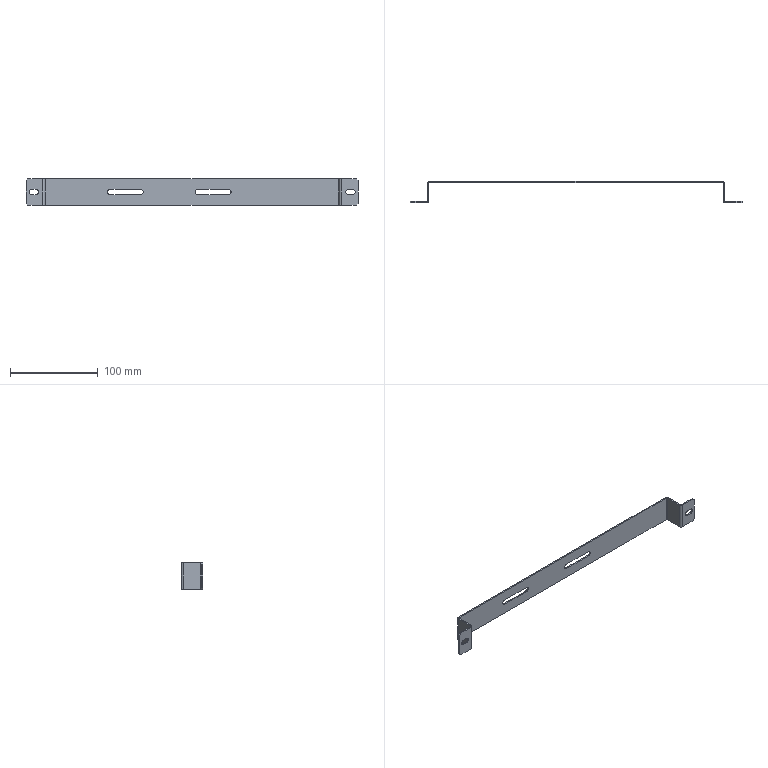Part | SolidWorks | features ICE 2, Chamfer 1, FlatPattern 1, SMBaseFlange 1, SheetMetal 1 | 1 solid | 58 faces | box 378 x 24.5 x 30 mm | volume 18043 mm3 | plane 42 | cylinder 16 | commonest cylinder face diameters 6 x8 2 x4 5 x4
STEP:
#1=CARTESIAN_POINT('',(0.,1.,30.));
#2=VERTEX_POINT('',#1);
#3=CARTESIAN_POINT('',(1.5,1.,30.));
#4=VERTEX_POINT('',#3);
#5=CARTESIAN_POINT('',(0.,1.,30.));
#6=DIRECTION('',(1.,0.,0.));
#7=VECTOR('',#6,1000.);
#8=LINE('',#5,#7);
#9=EDGE_CURVE('',#2,#4,#8,.T.);
#10=ORIENTED_EDGE('',*,*,#9,.F.);
#11=CARTESIAN_POINT('',(-1.,0.,30.));
#12=VERTEX_POINT('',#11);
#13=CARTESIAN_POINT('',(-1.,1.,30.));
#14=DIRECTION('',(0.,0.,1.));
#15=DIRECTION('',(-1.,0.,0.));
#16=AXIS2_PLACEMENT_3D('',#13,#14,#15);
#17=CIRCLE('',#16,1.);
#18=EDGE_CURVE('',#12,#2,#17,.T.);
#19=ORIENTED_EDGE('',*,*,#18,.F.);
#20=CARTESIAN_POINT('',(-1.,-1.5,30.));
#21=VERTEX_POINT('',#20);
#22=CARTESIAN_POINT('',(-1.,-1.5,30.));
#23=DIRECTION('',(0.,1.,0.));
#24=VECTOR('',#23,1000.);
#25=LINE('',#22,#24);
#26=EDGE_CURVE('',#21,#12,#25,.T.);
#27=ORIENTED_EDGE('',*,*,#26,.F.);
#28=CARTESIAN_POINT('',(-1.,1.,30.));
#29=DIRECTION('',(0.,0.,1.));
#30=DIRECTION('',(1.,0.,0.));
#31=AXIS2_PLACEMENT_3D('',#28,#29,#30);
#32=CIRCLE('',#31,2.5);
#33=EDGE_CURVE('',#21,#4,#32,.T.);
#34=ORIENTED_EDGE('',*,*,#33,.T.);
#35=EDGE_LOOP('',(#10,#19,#27,#34));
#36=FACE_OUTER_BOUND('',#35,.T.);
#37=CARTESIAN_POINT('',(0.,1.,30.));
#38=DIRECTION('',(0.,0.,1.));
#39=DIRECTION('',(1.,0.,0.));
#40=AXIS2_PLACEMENT_3D('',#37,#38,#39);
#41=PLANE('',#40);
#42=ADVANCED_FACE('',(#36),#41,.T.);
#43=CARTESIAN_POINT('',(0.,20.5,30.));
#44=VERTEX_POINT('',#43);
#45=CARTESIAN_POINT('',(0.,0.,30.));
#46=DIRECTION('',(0.,1.,0.));
#47=VECTOR('',#46,1000.);
#48=LINE('',#45,#47);
#49=EDGE_CURVE('',#2,#44,#48,.T.);
#50=ORIENTED_EDGE('',*,*,#49,.F.);
#51=ORIENTED_EDGE('',*,*,#9,.T.);
#52=CARTESIAN_POINT('',(1.5,20.5,30.));
#53=VERTEX_POINT('',#52);
#54=CARTESIAN_POINT('',(1.5,0.,30.));
#55=DIRECTION('',(0.,1.,0.));
#56=VECTOR('',#55,1000.);
#57=LINE('',#54,#56);
#58=EDGE_CURVE('',#4,#53,#57,.T.);
#59=ORIENTED_EDGE('',*,*,#58,.T.);
#60=CARTESIAN_POINT('',(1.5,20.5,30.));
#61=DIRECTION('',(-1.,0.,0.));
#62=VECTOR('',#61,1000.);
#63=LINE('',#60,#62);
#64=EDGE_CURVE('',#53,#44,#63,.T.);
#65=ORIENTED_EDGE('',*,*,#64,.T.);
#66=EDGE_LOOP('',(#50,#51,#59,#65));
#67=FACE_OUTER_BOUND('',#66,.T.);
#68=CARTESIAN_POINT('',(-1.,-1.5,30.));
#69=DIRECTION('',(0.,0.,1.));
#70=DIRECTION('',(1.,0.,0.));
#71=AXIS2_PLACEMENT_3D('',#68,#69,#70);
#72=PLANE('',#71);
#73=ADVANCED_FACE('',(#67),#72,.T.);
#74=CARTESIAN_POINT('',(-1.,0.,0.));
#75=VERTEX_POINT('',#74);
#76=CARTESIAN_POINT('',(-1.,-1.5,0.));
#77=VERTEX_POINT('',#76);
#78=CARTESIAN_POINT('',(-1.,0.,0.));
#79=DIRECTION('',(0.,-1.,0.));
#80=VECTOR('',#79,1000.);
#81=LINE('',#78,#80);
#82=EDGE_CURVE('',#75,#77,#81,.T.);
#83=ORIENTED_EDGE('',*,*,#82,.F.);
#84=CARTESIAN_POINT('',(0.,1.,0.));
#85=VERTEX_POINT('',#84);
#86=CARTESIAN_POINT('',(-1.,1.,0.));
#87=DIRECTION('',(0.,0.,1.));
#88=DIRECTION('',(-1.,0.,0.));
#89=AXIS2_PLACEMENT_3D('',#86,#87,#88);
#90=CIRCLE('',#89,1.);
#91=EDGE_CURVE('',#75,#85,#90,.T.);
#92=ORIENTED_EDGE('',*,*,#91,.T.);
#93=CARTESIAN_POINT('',(1.5,1.,0.));
#94=VERTEX_POINT('',#93);
#95=CARTESIAN_POINT('',(1.5,1.,0.));
#96=DIRECTION('',(-1.,0.,0.));
#97=VECTOR('',#96,1000.);
#98=LINE('',#95,#97);
#99=EDGE_CURVE('',#94,#85,#98,.T.);
#100=ORIENTED_EDGE('',*,*,#99,.F.);
#101=CARTESIAN_POINT('',(-1.,1.,0.));
#102=DIRECTION('',(0.,0.,1.));
#103=DIRECTION('',(1.,0.,0.));
#104=AXIS2_PLACEMENT_3D('',#101,#102,#103);
#105=CIRCLE('',#104,2.5);
#106=EDGE_CURVE('',#77,#94,#105,.T.);
#107=ORIENTED_EDGE('',*,*,#106,.F.);
#108=EDGE_LOOP('',(#83,#92,#100,#107));
#109=FACE_OUTER_BOUND('',#108,.T.);
#110=CARTESIAN_POINT('',(-1.,0.,0.));
#111=DIRECTION('',(0.,0.,-1.));
#112=DIRECTION('',(-1.,0.,0.));
#113=AXIS2_PLACEMENT_3D('',#110,#111,#112);
#114=PLANE('',#113);
#115=ADVANCED_FACE('',(#109),#114,.T.);
#116=CARTESIAN_POINT('',(-18.,-1.5,0.));
#117=VERTEX_POINT('',#116);
#118=CARTESIAN_POINT('',(-20.,-1.5,0.));
#119=DIRECTION('',(1.,0.,0.));
#120=VECTOR('',#119,1000.);
#121=LINE('',#118,#120);
#122=EDGE_CURVE('',#117,#77,#121,.T.);
#123=ORIENTED_EDGE('',*,*,#122,.F.);
#124=CARTESIAN_POINT('',(-18.,0.,0.));
#125=VERTEX_POINT('',#124);
#126=CARTESIAN_POINT('',(-18.,1.,0.));
#127=DIRECTION('',(0.,1.,0.));
#128=VECTOR('',#127,1000.);
#129=LINE('',#126,#128);
#130=EDGE_CURVE('',#117,#125,#129,.T.);
#131=ORIENTED_EDGE('',*,*,#130,.T.);
#132=CARTESIAN_POINT('',(-20.,0.,0.));
#133=DIRECTION('',(1.,0.,0.));
#134=VECTOR('',#133,1000.);
#135=LINE('',#132,#134);
#136=EDGE_CURVE('',#125,#75,#135,.T.);
#137=ORIENTED_EDGE('',*,*,#136,.T.);
#138=ORIENTED_EDGE('',*,*,#82,.T.);
#139=EDGE_LOOP('',(#123,#131,#137,#138));
#140=FACE_OUTER_BOUND('',#139,.T.);
#141=CARTESIAN_POINT('',(1.5,1.,0.));
#142=DIRECTION('',(0.,0.,-1.));
#143=DIRECTION('',(-1.,0.,0.));
#144=AXIS2_PLACEMENT_3D('',#141,#142,#143);
#145=PLANE('',#144);
#146=ADVANCED_FACE('',(#140),#145,.T.);
#147=CARTESIAN_POINT('',(2.5,23.,30.));
#148=VERTEX_POINT('',#147);
#149=CARTESIAN_POINT('',(2.5,21.5,30.));
#150=VERTEX_POINT('',#149);
#151=CARTESIAN_POINT('',(2.5,23.,30.));
#152=DIRECTION('',(0.,-1.,0.));
#153=VECTOR('',#152,1000.);
#154=LINE('',#151,#153);
#155=EDGE_CURVE('',#148,#150,#154,.T.);
#156=ORIENTED_EDGE('',*,*,#155,.F.);
#157=CARTESIAN_POINT('',(2.5,20.5,30.));
#158=DIRECTION('',(0.,0.,-1.));
#159=DIRECTION('',(1.,0.,0.));
#160=AXIS2_PLACEMENT_3D('',#157,#158,#159);
#161=CIRCLE('',#160,2.5);
#162=EDGE_CURVE('',#44,#148,#161,.T.);
#163=ORIENTED_EDGE('',*,*,#162,.F.);
#164=ORIENTED_EDGE('',*,*,#64,.F.);
#165=CARTESIAN_POINT('',(2.5,20.5,30.));
#166=DIRECTION('',(0.,0.,-1.));
#167=DIRECTION('',(1.,0.,0.));
#168=AXIS2_PLACEMENT_3D('',#165,#166,#167);
#169=CIRCLE('',#168,1.);
#170=EDGE_CURVE('',#53,#150,#169,.T.);
#171=ORIENTED_EDGE('',*,*,#170,.T.);
#172=EDGE_LOOP('',(#156,#163,#164,#171));
#173=FACE_OUTER_BOUND('',#172,.T.);
#174=CARTESIAN_POINT('',(2.5,23.,30.));
#175=DIRECTION('',(0.,0.,1.));
#176=DIRECTION('',(1.,0.,0.));
#177=AXIS2_PLACEMENT_3D('',#174,#175,#176);
#178=PLANE('',#177);
#179=ADVANCED_FACE('',(#173),#178,.T.);
#180=CARTESIAN_POINT('',(335.5,23.,30.));
#181=VERTEX_POINT('',#180);
#182=CARTESIAN_POINT('',(0.,23.,30.));
#183=DIRECTION('',(1.,0.,0.));
#184=VECTOR('',#183,1000.);
#185=LINE('',#182,#184);
#186=EDGE_CURVE('',#148,#181,#185,.T.);
#187=ORIENTED_EDGE('',*,*,#186,.F.);
#188=ORIENTED_EDGE('',*,*,#155,.T.);
#189=CARTESIAN_POINT('',(335.5,21.5,30.));
#190=VERTEX_POINT('',#189);
#191=CARTESIAN_POINT('',(0.,21.5,30.));
#192=DIRECTION('',(1.,0.,0.));
#193=VECTOR('',#192,1000.);
#194=LINE('',#191,#193);
#195=EDGE_CURVE('',#150,#190,#194,.T.);
#196=ORIENTED_EDGE('',*,*,#195,.T.);
#197=CARTESIAN_POINT('',(335.5,21.5,30.));
#198=DIRECTION('',(0.,1.,0.));
#199=VECTOR('',#198,1000.);
#200=LINE('',#197,#199);
#201=EDGE_CURVE('',#190,#181,#200,.T.);
#202=ORIENTED_EDGE('',*,*,#201,.T.);
#203=EDGE_LOOP('',(#187,#188,#196,#202));
#204=FACE_OUTER_BOUND('',#203,.T.);
#205=CARTESIAN_POINT('',(1.5,20.5,30.));
#206=DIRECTION('',(0.,0.,1.));
#207=DIRECTION('',(1.,0.,0.));
#208=AXIS2_PLACEMENT_3D('',#205,#206,#207);
#209=PLANE('',#208);
#210=ADVANCED_FACE('',(#204),#209,.T.);
#211=CARTESIAN_POINT('',(0.,20.5,0.));
#212=VERTEX_POINT('',#211);
#213=CARTESIAN_POINT('',(1.5,20.5,0.));
#214=VERTEX_POINT('',#213);
#215=CARTESIAN_POINT('',(0.,20.5,0.));
#216=DIRECTION('',(1.,0.,0.));
#217=VECTOR('',#216,1000.);
#218=LINE('',#215,#217);
#219=EDGE_CURVE('',#212,#214,#218,.T.);
#220=ORIENTED_EDGE('',*,*,#219,.F.);
#221=CARTESIAN_POINT('',(2.5,23.,0.));
#222=VERTEX_POINT('',#221);
#223=CARTESIAN_POINT('',(2.5,20.5,0.));
#224=DIRECTION('',(0.,0.,-1.));
#225=DIRECTION('',(1.,0.,0.));
#226=AXIS2_PLACEMENT_3D('',#223,#224,#225);
#227=CIRCLE('',#226,2.5);
#228=EDGE_CURVE('',#212,#222,#227,.T.);
#229=ORIENTED_EDGE('',*,*,#228,.T.);
#230=CARTESIAN_POINT('',(2.5,21.5,0.));
#231=VERTEX_POINT('',#230);
#232=CARTESIAN_POINT('',(2.5,21.5,0.));
#233=DIRECTION('',(0.,1.,0.));
#234=VECTOR('',#233,1000.);
#235=LINE('',#232,#234);
#236=EDGE_CURVE('',#231,#222,#235,.T.);
#237=ORIENTED_EDGE('',*,*,#236,.F.);
#238=CARTESIAN_POINT('',(2.5,20.5,0.));
#239=DIRECTION('',(0.,0.,-1.));
#240=DIRECTION('',(1.,0.,0.));
#241=AXIS2_PLACEMENT_3D('',#238,#239,#240);
#242=CIRCLE('',#241,1.);
#243=EDGE_CURVE('',#214,#231,#242,.T.);
#244=ORIENTED_EDGE('',*,*,#243,.F.);
#245=EDGE_LOOP('',(#220,#229,#237,#244));
#246=FACE_OUTER_BOUND('',#245,.T.);
#247=CARTESIAN_POINT('',(0.,20.5,0.));
#248=DIRECTION('',(0.,0.,-1.));
#249=DIRECTION('',(-1.,0.,0.));
#250=AXIS2_PLACEMENT_3D('',#247,#248,#249);
#251=PLANE('',#250);
#252=ADVANCED_FACE('',(#246),#251,.T.);
#253=CARTESIAN_POINT('',(0.,0.,0.));
#254=DIRECTION('',(0.,1.,0.));
#255=VECTOR('',#254,1000.);
#256=LINE('',#253,#255);
#257=EDGE_CURVE('',#85,#212,#256,.T.);
#258=ORIENTED_EDGE('',*,*,#257,.T.);
#259=ORIENTED_EDGE('',*,*,#219,.T.);
#260=CARTESIAN_POINT('',(1.5,0.,0.));
#261=DIRECTION('',(0.,1.,0.));
#262=VECTOR('',#261,1000.);
#263=LINE('',#260,#262);
#264=EDGE_CURVE('',#94,#214,#263,.T.);
#265=ORIENTED_EDGE('',*,*,#264,.F.);
#266=ORIENTED_EDGE('',*,*,#99,.T.);
#267=EDGE_LOOP('',(#258,#259,#265,#266));
#268=FACE_OUTER_BOUND('',#267,.T.);
#269=CARTESIAN_POINT('',(2.5,21.5,0.));
#270=DIRECTION('',(0.,0.,-1.));
#271=DIRECTION('',(-1.,0.,0.));
#272=AXIS2_PLACEMENT_3D('',#269,#270,#271);
#273=PLANE('',#272);
#274=ADVANCED_FACE('',(#268),#273,.T.);
#275=CARTESIAN_POINT('',(338.,20.5,30.));
#276=VERTEX_POINT('',#275);
#277=CARTESIAN_POINT('',(336.5,20.5,30.));
#278=VERTEX_POINT('',#277);
#279=CARTESIAN_POINT('',(338.,20.5,30.));
#280=DIRECTION('',(-1.,0.,0.));
#281=VECTOR('',#280,1000.);
#282=LINE('',#279,#281);
#283=EDGE_CURVE('',#276,#278,#282,.T.);
#284=ORIENTED_EDGE('',*,*,#283,.F.);
#285=CARTESIAN_POINT('',(335.5,20.5,30.));
#286=DIRECTION('',(0.,0.,-1.));
#287=DIRECTION('',(1.,0.,0.));
#288=AXIS2_PLACEMENT_3D('',#285,#286,#287);
#289=CIRCLE('',#288,2.5);
#290=EDGE_CURVE('',#181,#276,#289,.T.);
#291=ORIENTED_EDGE('',*,*,#290,.F.);
#292=ORIENTED_EDGE('',*,*,#201,.F.);
#293=CARTESIAN_POINT('',(335.5,20.5,30.));
#294=DIRECTION('',(0.,0.,-1.));
#295=DIRECTION('',(1.,0.,0.));
#296=AXIS2_PLACEMENT_3D('',#293,#294,#295);
#297=CIRCLE('',#296,1.);
#298=EDGE_CURVE('',#190,#278,#297,.T.);
#299=ORIENTED_EDGE('',*,*,#298,.T.);
#300=EDGE_LOOP('',(#284,#291,#292,#299));
#301=FACE_OUTER_BOUND('',#300,.T.);
#302=CARTESIAN_POINT('',(338.,20.5,30.));
#303=DIRECTION('',(0.,0.,1.));
#304=DIRECTION('',(1.,0.,0.));
#305=AXIS2_PLACEMENT_3D('',#302,#303,#304);
#306=PLANE('',#305);
#307=ADVANCED_FACE('',(#301),#306,.T.);
#308=CARTESIAN_POINT('',(338.,1.,30.));
#309=VERTEX_POINT('',#308);
#310=CARTESIAN_POINT('',(338.,23.,30.));
#311=DIRECTION('',(0.,-1.,0.));
#312=VECTOR('',#311,1000.);
#313=LINE('',#310,#312);
#314=EDGE_CURVE('',#276,#309,#313,.T.);
#315=ORIENTED_EDGE('',*,*,#314,.F.);
#316=ORIENTED_EDGE('',*,*,#283,.T.);
#317=CARTESIAN_POINT('',(336.5,1.,30.));
#318=VERTEX_POINT('',#317);
#319=CARTESIAN_POINT('',(336.5,23.,30.));
#320=DIRECTION('',(0.,-1.,0.));
#321=VECTOR('',#320,1000.);
#322=LINE('',#319,#321);
#323=EDGE_CURVE('',#278,#318,#322,.T.);
#324=ORIENTED_EDGE('',*,*,#323,.T.);
#325=CARTESIAN_POINT('',(336.5,1.,30.));
#326=DIRECTION('',(1.,0.,0.));
#327=VECTOR('',#326,1000.);
#328=LINE('',#325,#327);
#329=EDGE_CURVE('',#318,#309,#328,.T.);
#330=ORIENTED_EDGE('',*,*,#329,.T.);
#331=EDGE_LOOP('',(#315,#316,#324,#330));
#332=FACE_OUTER_BOUND('',#331,.T.);
#333=CARTESIAN_POINT('',(335.5,21.5,30.));
#334=DIRECTION('',(0.,0.,1.));
#335=DIRECTION('',(1.,0.,0.));
#336=AXIS2_PLACEMENT_3D('',#333,#334,#335);
#337=PLANE('',#336);
#338=ADVANCED_FACE('',(#332),#337,.T.);
#339=CARTESIAN_POINT('',(335.5,23.,0.));
#340=VERTEX_POINT('',#339);
#341=CARTESIAN_POINT('',(335.5,21.5,0.));
#342=VERTEX_POINT('',#341);
#343=CARTESIAN_POINT('',(335.5,23.,0.));
#344=DIRECTION('',(0.,-1.,0.));
#345=VECTOR('',#344,1000.);
#346=LINE('',#343,#345);
#347=EDGE_CURVE('',#340,#342,#346,.T.);
#348=ORIENTED_EDGE('',*,*,#347,.F.);
#349=CARTESIAN_POINT('',(338.,20.5,0.));
#350=VERTEX_POINT('',#349);
#351=CARTESIAN_POINT('',(335.5,20.5,0.));
#352=DIRECTION('',(0.,0.,-1.));
#353=DIRECTION('',(1.,0.,0.));
#354=AXIS2_PLACEMENT_3D('',#351,#352,#353);
#355=CIRCLE('',#354,2.5);
#356=EDGE_CURVE('',#340,#350,#355,.T.);
#357=ORIENTED_EDGE('',*,*,#356,.T.);
#358=CARTESIAN_POINT('',(336.5,20.5,0.));
#359=VERTEX_POINT('',#358);
#360=CARTESIAN_POINT('',(336.5,20.5,0.));
#361=DIRECTION('',(1.,0.,0.));
#362=VECTOR('',#361,1000.);
#363=LINE('',#360,#362);
#364=EDGE_CURVE('',#359,#350,#363,.T.);
#365=ORIENTED_EDGE('',*,*,#364,.F.);
#366=CARTESIAN_POINT('',(335.5,20.5,0.));
#367=DIRECTION('',(0.,0.,-1.));
#368=DIRECTION('',(1.,0.,0.));
#369=AXIS2_PLACEMENT_3D('',#366,#367,#368);
#370=CIRCLE('',#369,1.);
#371=EDGE_CURVE('',#342,#359,#370,.T.);
#372=ORIENTED_EDGE('',*,*,#371,.F.);
#373=EDGE_LOOP('',(#348,#357,#365,#372));
#374=FACE_OUTER_BOUND('',#373,.T.);
#375=CARTESIAN_POINT('',(335.5,23.,0.));
#376=DIRECTION('',(0.,0.,-1.));
#377=DIRECTION('',(-1.,0.,0.));
#378=AXIS2_PLACEMENT_3D('',#375,#376,#377);
#379=PLANE('',#378);
#380=ADVANCED_FACE('',(#374),#379,.T.);
#381=CARTESIAN_POINT('',(0.,23.,0.));
#382=DIRECTION('',(1.,0.,0.));
#383=VECTOR('',#382,1000.);
#384=LINE('',#381,#383);
#385=EDGE_CURVE('',#222,#340,#384,.T.);
#386=ORIENTED_EDGE('',*,*,#385,.T.);
#387=ORIENTED_EDGE('',*,*,#347,.T.);
#388=CARTESIAN_POINT('',(0.,21.5,0.));
#389=DIRECTION('',(1.,0.,0.));
#390=VECTOR('',#389,1000.);
#391=LINE('',#388,#390);
#392=EDGE_CURVE('',#231,#342,#391,.T.);
#393=ORIENTED_EDGE('',*,*,#392,.F.);
#394=ORIENTED_EDGE('',*,*,#236,.T.);
#395=EDGE_LOOP('',(#386,#387,#393,#394));
#396=FACE_OUTER_BOUND('',#395,.T.);
#397=CARTESIAN_POINT('',(336.5,20.5,0.));
#398=DIRECTION('',(0.,0.,-1.));
#399=DIRECTION('',(-1.,0.,0.));
#400=AXIS2_PLACEMENT_3D('',#397,#398,#399);
#401=PLANE('',#400);
#402=ADVANCED_FACE('',(#396),#401,.T.);
#403=CARTESIAN_POINT('',(339.,0.,30.));
#404=VERTEX_POINT('',#403);
#405=CARTESIAN_POINT('',(339.,-1.5,30.));
#406=VERTEX_POINT('',#405);
#407=CARTESIAN_POINT('',(339.,0.,30.));
#408=DIRECTION('',(0.,-1.,0.));
#409=VECTOR('',#408,1000.);
#410=LINE('',#407,#409);
#411=EDGE_CURVE('',#404,#406,#410,.T.);
#412=ORIENTED_EDGE('',*,*,#411,.F.);
#413=CARTESIAN_POINT('',(339.,1.,30.));
#414=DIRECTION('',(0.,0.,1.));
#415=DIRECTION('',(-1.,0.,0.));
#416=AXIS2_PLACEMENT_3D('',#413,#414,#415);
#417=CIRCLE('',#416,1.);
#418=EDGE_CURVE('',#309,#404,#417,.T.);
#419=ORIENTED_EDGE('',*,*,#418,.F.);
#420=ORIENTED_EDGE('',*,*,#329,.F.);
#421=CARTESIAN_POINT('',(339.,1.,30.));
#422=DIRECTION('',(0.,0.,1.));
#423=DIRECTION('',(1.,0.,0.));
#424=AXIS2_PLACEMENT_3D('',#421,#422,#423);
#425=CIRCLE('',#424,2.5);
#426=EDGE_CURVE('',#318,#406,#425,.T.);
#427=ORIENTED_EDGE('',*,*,#426,.T.);
#428=EDGE_LOOP('',(#412,#419,#420,#427));
#429=FACE_OUTER_BOUND('',#428,.T.);
#430=CARTESIAN_POINT('',(339.,0.,30.));
#431=DIRECTION('',(0.,0.,1.));
#432=DIRECTION('',(1.,0.,0.));
#433=AXIS2_PLACEMENT_3D('',#430,#431,#432);
#434=PLANE('',#433);
#435=ADVANCED_FACE('',(#429),#434,.T.);
#436=CARTESIAN_POINT('',(356.,-1.5,30.));
#437=VERTEX_POINT('',#436);
#438=CARTESIAN_POINT('',(338.,-1.5,30.));
#439=DIRECTION('',(1.,0.,0.));
#440=VECTOR('',#439,1000.);
#441=LINE('',#438,#440);
#442=EDGE_CURVE('',#406,#437,#441,.T.);
#443=ORIENTED_EDGE('',*,*,#442,.T.);
#444=CARTESIAN_POINT('',(356.,0.,30.));
#445=VERTEX_POINT('',#444);
#446=CARTESIAN_POINT('',(356.,1.,30.));
#447=DIRECTION('',(0.,1.,0.));
#448=VECTOR('',#447,1000.);
#449=LINE('',#446,#448);
#450=EDGE_CURVE('',#437,#445,#449,.T.);
#451=ORIENTED_EDGE('',*,*,#450,.T.);
#452=CARTESIAN_POINT('',(338.,0.,30.));
#453=DIRECTION('',(1.,0.,0.));
#454=VECTOR('',#453,1000.);
#455=LINE('',#452,#454);
#456=EDGE_CURVE('',#404,#445,#455,.T.);
#457=ORIENTED_EDGE('',*,*,#456,.F.);
#458=ORIENTED_EDGE('',*,*,#411,.T.);
#459=EDGE_LOOP('',(#443,#451,#457,#458));
#460=FACE_OUTER_BOUND('',#459,.T.);
#461=CARTESIAN_POINT('',(336.5,1.,30.));
#462=DIRECTION('',(0.,0.,1.));
#463=DIRECTION('',(1.,0.,0.));
#464=AXIS2_PLACEMENT_3D('',#461,#462,#463);
#465=PLANE('',#464);
#466=ADVANCED_FACE('',(#460),#465,.T.);
#467=CARTESIAN_POINT('',(338.,1.,0.));
#468=VERTEX_POINT('',#467);
#469=CARTESIAN_POINT('',(336.5,1.,0.));
#470=VERTEX_POINT('',#469);
#471=CARTESIAN_POINT('',(338.,1.,0.));
#472=DIRECTION('',(-1.,0.,0.));
#473=VECTOR('',#472,1000.);
#474=LINE('',#471,#473);
#475=EDGE_CURVE('',#468,#470,#474,.T.);
#476=ORIENTED_EDGE('',*,*,#475,.F.);
#477=CARTESIAN_POINT('',(339.,0.,0.));
#478=VERTEX_POINT('',#477);
#479=CARTESIAN_POINT('',(339.,1.,0.));
#480=DIRECTION('',(0.,0.,1.));
#481=DIRECTION('',(-1.,0.,0.));
#482=AXIS2_PLACEMENT_3D('',#479,#480,#481);
#483=CIRCLE('',#482,1.);
#484=EDGE_CURVE('',#468,#478,#483,.T.);
#485=ORIENTED_EDGE('',*,*,#484,.T.);
#486=CARTESIAN_POINT('',(339.,-1.5,0.));
#487=VERTEX_POINT('',#486);
#488=CARTESIAN_POINT('',(339.,-1.5,0.));
#489=DIRECTION('',(0.,1.,0.));
#490=VECTOR('',#489,1000.);
#491=LINE('',#488,#490);
#492=EDGE_CURVE('',#487,#478,#491,.T.);
#493=ORIENTED_EDGE('',*,*,#492,.F.);
#494=CARTESIAN_POINT('',(339.,1.,0.));
#495=DIRECTION('',(0.,0.,1.));
#496=DIRECTION('',(1.,0.,0.));
#497=AXIS2_PLACEMENT_3D('',#494,#495,#496);
#498=CIRCLE('',#497,2.5);
#499=EDGE_CURVE('',#470,#487,#498,.T.);
#500=ORIENTED_EDGE('',*,*,#499,.F.);
#501=EDGE_LOOP('',(#476,#485,#493,#500));
#502=FACE_OUTER_BOUND('',#501,.T.);
#503=CARTESIAN_POINT('',(338.,1.,0.));
#504=DIRECTION('',(0.,0.,-1.));
#505=DIRECTION('',(-1.,0.,0.));
#506=AXIS2_PLACEMENT_3D('',#503,#504,#505);
#507=PLANE('',#506);
#508=ADVANCED_FACE('',(#502),#507,.T.);
#509=CARTESIAN_POINT('',(338.,23.,0.));
#510=DIRECTION('',(0.,-1.,0.));
#511=VECTOR('',#510,1000.);
#512=LINE('',#509,#511);
#513=EDGE_CURVE('',#350,#468,#512,.T.);
#514=ORIENTED_EDGE('',*,*,#513,.T.);
#515=ORIENTED_EDGE('',*,*,#475,.T.);
#516=CARTESIAN_POINT('',(336.5,23.,0.));
#517=DIRECTION('',(0.,-1.,0.));
#518=VECTOR('',#517,1000.);
#519=LINE('',#516,#518);
#520=EDGE_CURVE('',#359,#470,#519,.T.);
#521=ORIENTED_EDGE('',*,*,#520,.F.);
#522=ORIENTED_EDGE('',*,*,#364,.T.);
#523=EDGE_LOOP('',(#514,#515,#521,#522));
#524=FACE_OUTER_BOUND('',#523,.T.);
#525=CARTESIAN_POINT('',(339.,-1.5,0.));
#526=DIRECTION('',(0.,0.,-1.));
#527=DIRECTION('',(-1.,0.,0.));
#528=AXIS2_PLACEMENT_3D('',#525,#526,#527);
#529=PLANE('',#528);
#530=ADVANCED_FACE('',(#524),#529,.T.);
#531=CARTESIAN_POINT('',(347.,-1.5,12.));
#532=VERTEX_POINT('',#531);
#533=CARTESIAN_POINT('',(347.,-1.5,18.));
#534=VERTEX_POINT('',#533);
#535=CARTESIAN_POINT('',(347.,-1.5,15.));
#536=DIRECTION('',(0.,1.,0.));
#537=DIRECTION('',(0.,0.,1.));
#538=AXIS2_PLACEMENT_3D('',#535,#536,#537);
#539=CIRCLE('',#538,3.);
#540=EDGE_CURVE('',#532,#534,#539,.T.);
#541=ORIENTED_EDGE('',*,*,#540,.T.);
#542=CARTESIAN_POINT('',(352.,-1.5,18.));
#543=VERTEX_POINT('',#542);
#544=CARTESIAN_POINT('',(352.,-1.5,18.));
#545=DIRECTION('',(1.,0.,0.));
#546=VECTOR('',#545,1000.);
#547=LINE('',#544,#546);
#548=EDGE_CURVE('',#534,#543,#547,.T.);
#549=ORIENTED_EDGE('',*,*,#548,.T.);
#550=CARTESIAN_POINT('',(352.,-1.5,12.));
#551=VERTEX_POINT('',#550);
#552=CARTESIAN_POINT('',(352.,-1.5,15.));
#553=DIRECTION('',(0.,1.,0.));
#554=DIRECTION('',(0.,0.,1.));
#555=AXIS2_PLACEMENT_3D('',#552,#553,#554);
#556=CIRCLE('',#555,3.);
#557=EDGE_CURVE('',#543,#551,#556,.T.);
#558=ORIENTED_EDGE('',*,*,#557,.T.);
#559=CARTESIAN_POINT('',(352.,-1.5,12.));
#560=DIRECTION('',(-1.,0.,0.));
#561=VECTOR('',#560,1000.);
#562=LINE('',#559,#561);
#563=EDGE_CURVE('',#551,#532,#562,.T.);
#564=ORIENTED_EDGE('',*,*,#563,.T.);
#565=EDGE_LOOP('',(#541,#549,#558,#564));
#566=FACE_BOUND('',#565,.T.);
#567=CARTESIAN_POINT('',(356.,-1.5,0.));
#568=VERTEX_POINT('',#567);
#569=CARTESIAN_POINT('',(338.,-1.5,0.));
#570=DIRECTION('',(1.,0.,0.));
#571=VECTOR('',#570,1000.);
#572=LINE('',#569,#571);
#573=EDGE_CURVE('',#487,#568,#572,.T.);
#574=ORIENTED_EDGE('',*,*,#573,.T.);
#575=CARTESIAN_POINT('',(358.,-1.5,2.));
#576=VERTEX_POINT('',#575);
#577=CARTESIAN_POINT('',(356.,-1.5,0.));
#578=DIRECTION('',(0.7071,0.,0.7071));
#579=VECTOR('',#578,1000.);
#580=LINE('',#577,#579);
#581=EDGE_CURVE('',#568,#576,#580,.T.);
#582=ORIENTED_EDGE('',*,*,#581,.T.);
#583=CARTESIAN_POINT('',(358.,-1.5,28.));
#584=VERTEX_POINT('',#583);
#585=CARTESIAN_POINT('',(358.,-1.5,30.));
#586=DIRECTION('',(0.,0.,-1.));
#587=VECTOR('',#586,1000.);
#588=LINE('',#585,#587);
#589=EDGE_CURVE('',#584,#576,#588,.T.);
#590=ORIENTED_EDGE('',*,*,#589,.F.);
#591=CARTESIAN_POINT('',(358.,-1.5,28.));
#592=DIRECTION('',(-0.7071,0.,0.7071));
#593=VECTOR('',#592,1000.);
#594=LINE('',#591,#593);
#595=EDGE_CURVE('',#584,#437,#594,.T.);
#596=ORIENTED_EDGE('',*,*,#595,.T.);
#597=ORIENTED_EDGE('',*,*,#442,.F.);
#598=CARTESIAN_POINT('',(339.,-1.5,30.));
#599=DIRECTION('',(0.,0.,-1.));
#600=VECTOR('',#599,1000.);
#601=LINE('',#598,#600);
#602=EDGE_CURVE('',#406,#487,#601,.T.);
#603=ORIENTED_EDGE('',*,*,#602,.T.);
#604=EDGE_LOOP('',(#574,#582,#590,#596,#597,#603));
#605=FACE_OUTER_BOUND('',#604,.T.);
#606=CARTESIAN_POINT('',(338.,-1.5,30.));
#607=DIRECTION('',(0.,1.,0.));
#608=DIRECTION('',(0.,0.,1.));
#609=AXIS2_PLACEMENT_3D('',#606,#607,#608);
#610=PLANE('',#609);
#611=ADVANCED_FACE('',(#566,#605),#610,.F.);
#612=ORIENTED_EDGE('',*,*,#589,.T.);
#613=CARTESIAN_POINT('',(358.,0.,2.));
#614=VERTEX_POINT('',#613);
#615=CARTESIAN_POINT('',(358.,0.,2.));
#616=DIRECTION('',(0.,1.,0.));
#617=VECTOR('',#616,1000.);
#618=LINE('',#615,#617);
#619=EDGE_CURVE('',#576,#614,#618,.T.);
#620=ORIENTED_EDGE('',*,*,#619,.T.);
#621=CARTESIAN_POINT('',(358.,0.,28.));
#622=VERTEX_POINT('',#621);
#623=CARTESIAN_POINT('',(358.,0.,30.));
#624=DIRECTION('',(0.,0.,-1.));
#625=VECTOR('',#624,1000.);
#626=LINE('',#623,#625);
#627=EDGE_CURVE('',#622,#614,#626,.T.);
#628=ORIENTED_EDGE('',*,*,#627,.F.);
#629=CARTESIAN_POINT('',(358.,0.,28.));
#630=DIRECTION('',(0.,-1.,0.));
#631=VECTOR('',#630,1000.);
#632=LINE('',#629,#631);
#633=EDGE_CURVE('',#622,#584,#632,.T.);
#634=ORIENTED_EDGE('',*,*,#633,.T.);
#635=EDGE_LOOP('',(#612,#620,#628,#634));
#636=FACE_OUTER_BOUND('',#635,.T.);
#637=CARTESIAN_POINT('',(358.,0.,30.));
#638=DIRECTION('',(1.,0.,0.));
#639=DIRECTION('',(0.,0.,-1.));
#640=AXIS2_PLACEMENT_3D('',#637,#638,#639);
#641=PLANE('',#640);
#642=ADVANCED_FACE('',(#636),#641,.T.);
#643=CARTESIAN_POINT('',(352.,0.,18.));
#644=VERTEX_POINT('',#643);
#645=CARTESIAN_POINT('',(352.,0.,12.));
#646=VERTEX_POINT('',#645);
#647=CARTESIAN_POINT('',(352.,0.,15.));
#648=DIRECTION('',(0.,1.,0.));
#649=DIRECTION('',(0.,0.,1.));
#650=AXIS2_PLACEMENT_3D('',#647,#648,#649);
#651=CIRCLE('',#650,3.);
#652=EDGE_CURVE('',#644,#646,#651,.T.);
#653=ORIENTED_EDGE('',*,*,#652,.F.);
#654=CARTESIAN_POINT('',(347.,0.,18.));
#655=VERTEX_POINT('',#654);
#656=CARTESIAN_POINT('',(352.,0.,18.));
#657=DIRECTION('',(1.,0.,0.));
#658=VECTOR('',#657,1000.);
#659=LINE('',#656,#658);
#660=EDGE_CURVE('',#655,#644,#659,.T.);
#661=ORIENTED_EDGE('',*,*,#660,.F.);
#662=CARTESIAN_POINT('',(347.,0.,12.));
#663=VERTEX_POINT('',#662);
#664=CARTESIAN_POINT('',(347.,0.,15.));
#665=DIRECTION('',(0.,1.,0.));
#666=DIRECTION('',(0.,0.,1.));
#667=AXIS2_PLACEMENT_3D('',#664,#665,#666);
#668=CIRCLE('',#667,3.);
#669=EDGE_CURVE('',#663,#655,#668,.T.);
#670=ORIENTED_EDGE('',*,*,#669,.F.);
#671=CARTESIAN_POINT('',(352.,0.,12.));
#672=DIRECTION('',(-1.,0.,0.));
#673=VECTOR('',#672,1000.);
#674=LINE('',#671,#673);
#675=EDGE_CURVE('',#646,#663,#674,.T.);
#676=ORIENTED_EDGE('',*,*,#675,.F.);
#677=EDGE_LOOP('',(#653,#661,#670,#676));
#678=FACE_BOUND('',#677,.T.);
#679=ORIENTED_EDGE('',*,*,#627,.T.);
#680=CARTESIAN_POINT('',(356.,0.,0.));
#681=VERTEX_POINT('',#680);
#682=CARTESIAN_POINT('',(362.,0.,6.));
#683=DIRECTION('',(-0.7071,0.,-0.7071));
#684=VECTOR('',#683,1000.);
#685=LINE('',#682,#684);
#686=EDGE_CURVE('',#614,#681,#685,.T.);
#687=ORIENTED_EDGE('',*,*,#686,.T.);
#688=CARTESIAN_POINT('',(338.,0.,0.));
#689=DIRECTION('',(1.,0.,0.));
#690=VECTOR('',#689,1000.);
#691=LINE('',#688,#690);
#692=EDGE_CURVE('',#478,#681,#691,.T.);
#693=ORIENTED_EDGE('',*,*,#692,.F.);
#694=CARTESIAN_POINT('',(339.,0.,30.));
#695=DIRECTION('',(0.,0.,-1.));
#696=VECTOR('',#695,1000.);
#697=LINE('',#694,#696);
#698=EDGE_CURVE('',#404,#478,#697,.T.);
#699=ORIENTED_EDGE('',*,*,#698,.F.);
#700=ORIENTED_EDGE('',*,*,#456,.T.);
#701=CARTESIAN_POINT('',(347.,0.,39.));
#702=DIRECTION('',(0.7071,0.,-0.7071));
#703=VECTOR('',#702,1000.);
#704=LINE('',#701,#703);
#705=EDGE_CURVE('',#445,#622,#704,.T.);
#706=ORIENTED_EDGE('',*,*,#705,.T.);
#707=EDGE_LOOP('',(#679,#687,#693,#699,#700,#706));
#708=FACE_OUTER_BOUND('',#707,.T.);
#709=CARTESIAN_POINT('',(338.,0.,30.));
#710=DIRECTION('',(0.,1.,0.));
#711=DIRECTION('',(0.,0.,1.));
#712=AXIS2_PLACEMENT_3D('',#709,#710,#711);
#713=PLANE('',#712);
#714=ADVANCED_FACE('',(#678,#708),#713,.T.);
#715=ORIENTED_EDGE('',*,*,#484,.F.);
#716=CARTESIAN_POINT('',(338.,1.,30.));
#717=DIRECTION('',(0.,0.,-1.));
#718=VECTOR('',#717,1000.);
#719=LINE('',#716,#718);
#720=EDGE_CURVE('',#309,#468,#719,.T.);
#721=ORIENTED_EDGE('',*,*,#720,.F.);
#722=ORIENTED_EDGE('',*,*,#418,.T.);
#723=ORIENTED_EDGE('',*,*,#698,.T.);
#724=EDGE_LOOP('',(#715,#721,#722,#723));
#725=FACE_OUTER_BOUND('',#724,.T.);
#726=CARTESIAN_POINT('',(339.,1.,30.));
#727=DIRECTION('',(0.,0.,-1.));
#728=DIRECTION('',(-1.,0.,0.));
#729=AXIS2_PLACEMENT_3D('',#726,#727,#728);
#730=CYLINDRICAL_SURFACE('',#729,1.);
#731=ADVANCED_FACE('',(#725),#730,.F.);
#732=ORIENTED_EDGE('',*,*,#513,.F.);
#733=CARTESIAN_POINT('',(338.,20.5,30.));
#734=DIRECTION('',(0.,0.,-1.));
#735=VECTOR('',#734,1000.);
#736=LINE('',#733,#735);
#737=EDGE_CURVE('',#276,#350,#736,.T.);
#738=ORIENTED_EDGE('',*,*,#737,.F.);
#739=ORIENTED_EDGE('',*,*,#314,.T.);
#740=ORIENTED_EDGE('',*,*,#720,.T.);
#741=EDGE_LOOP('',(#732,#738,#739,#740));
#742=FACE_OUTER_BOUND('',#741,.T.);
#743=CARTESIAN_POINT('',(338.,23.,30.));
#744=DIRECTION('',(1.,0.,0.));
#745=DIRECTION('',(0.,0.,-1.));
#746=AXIS2_PLACEMENT_3D('',#743,#744,#745);
#747=PLANE('',#746);
#748=ADVANCED_FACE('',(#742),#747,.T.);
#749=ORIENTED_EDGE('',*,*,#356,.F.);
#750=CARTESIAN_POINT('',(335.5,23.,30.));
#751=DIRECTION('',(0.,0.,-1.));
#752=VECTOR('',#751,1000.);
#753=LINE('',#750,#752);
#754=EDGE_CURVE('',#181,#340,#753,.T.);
#755=ORIENTED_EDGE('',*,*,#754,.F.);
#756=ORIENTED_EDGE('',*,*,#290,.T.);
#757=ORIENTED_EDGE('',*,*,#737,.T.);
#758=EDGE_LOOP('',(#749,#755,#756,#757));
#759=FACE_OUTER_BOUND('',#758,.T.);
#760=CARTESIAN_POINT('',(335.5,20.5,30.));
#761=DIRECTION('',(0.,0.,-1.));
#762=DIRECTION('',(-1.,0.,0.));
#763=AXIS2_PLACEMENT_3D('',#760,#761,#762);
#764=CYLINDRICAL_SURFACE('',#763,2.5);
#765=ADVANCED_FACE('',(#759),#764,.T.);
#766=CARTESIAN_POINT('',(175.5,23.,12.));
#767=VERTEX_POINT('',#766);
#768=CARTESIAN_POINT('',(175.5,23.,18.));
#769=VERTEX_POINT('',#768);
#770=CARTESIAN_POINT('',(175.5,23.,15.));
#771=DIRECTION('',(0.,1.,0.));
#772=DIRECTION('',(0.,0.,1.));
#773=AXIS2_PLACEMENT_3D('',#770,#771,#772);
#774=CIRCLE('',#773,3.);
#775=EDGE_CURVE('',#767,#769,#774,.T.);
#776=ORIENTED_EDGE('',*,*,#775,.F.);
#777=CARTESIAN_POINT('',(210.5,23.,12.));
#778=VERTEX_POINT('',#777);
#779=CARTESIAN_POINT('',(175.5,23.,12.));
#780=DIRECTION('',(-1.,0.,0.));
#781=VECTOR('',#780,1000.);
#782=LINE('',#779,#781);
#783=EDGE_CURVE('',#778,#767,#782,.T.);
#784=ORIENTED_EDGE('',*,*,#783,.F.);
#785=CARTESIAN_POINT('',(210.5,23.,18.));
#786=VERTEX_POINT('',#785);
#787=CARTESIAN_POINT('',(210.5,23.,15.));
#788=DIRECTION('',(0.,1.,0.));
#789=DIRECTION('',(0.,0.,1.));
#790=AXIS2_PLACEMENT_3D('',#787,#788,#789);
#791=CIRCLE('',#790,3.);
#792=EDGE_CURVE('',#786,#778,#791,.T.);
#793=ORIENTED_EDGE('',*,*,#792,.F.);
#794=CARTESIAN_POINT('',(175.5,23.,18.));
#795=DIRECTION('',(1.,0.,0.));
#796=VECTOR('',#795,1000.);
#797=LINE('',#794,#796);
#798=EDGE_CURVE('',#769,#786,#797,.T.);
#799=ORIENTED_EDGE('',*,*,#798,.F.);
#800=EDGE_LOOP('',(#776,#784,#793,#799));
#801=FACE_BOUND('',#800,.T.);
#802=CARTESIAN_POINT('',(75.5,23.,12.));
#803=VERTEX_POINT('',#802);
#804=CARTESIAN_POINT('',(75.5,23.,18.));
#805=VERTEX_POINT('',#804);
#806=CARTESIAN_POINT('',(75.5,23.,15.));
#807=DIRECTION('',(0.,1.,0.));
#808=DIRECTION('',(0.,0.,1.));
#809=AXIS2_PLACEMENT_3D('',#806,#807,#808);
#810=CIRCLE('',#809,3.);
#811=EDGE_CURVE('',#803,#805,#810,.T.);
#812=ORIENTED_EDGE('',*,*,#811,.F.);
#813=CARTESIAN_POINT('',(110.5,23.,12.));
#814=VERTEX_POINT('',#813);
#815=CARTESIAN_POINT('',(75.5,23.,12.));
#816=DIRECTION('',(-1.,0.,0.));
#817=VECTOR('',#816,1000.);
#818=LINE('',#815,#817);
#819=EDGE_CURVE('',#814,#803,#818,.T.);
#820=ORIENTED_EDGE('',*,*,#819,.F.);
#821=CARTESIAN_POINT('',(110.5,23.,18.));
#822=VERTEX_POINT('',#821);
#823=CARTESIAN_POINT('',(110.5,23.,15.));
#824=DIRECTION('',(0.,1.,0.));
#825=DIRECTION('',(0.,0.,1.));
#826=AXIS2_PLACEMENT_3D('',#823,#824,#825);
#827=CIRCLE('',#826,3.);
#828=EDGE_CURVE('',#822,#814,#827,.T.);
#829=ORIENTED_EDGE('',*,*,#828,.F.);
#830=CARTESIAN_POINT('',(75.5,23.,18.));
#831=DIRECTION('',(1.,0.,0.));
#832=VECTOR('',#831,1000.);
#833=LINE('',#830,#832);
#834=EDGE_CURVE('',#805,#822,#833,.T.);
#835=ORIENTED_EDGE('',*,*,#834,.F.);
#836=EDGE_LOOP('',(#812,#820,#829,#835));
#837=FACE_BOUND('',#836,.T.);
#838=ORIENTED_EDGE('',*,*,#385,.F.);
#839=CARTESIAN_POINT('',(2.5,23.,30.));
#840=DIRECTION('',(0.,0.,-1.));
#841=VECTOR('',#840,1000.);
#842=LINE('',#839,#841);
#843=EDGE_CURVE('',#148,#222,#842,.T.);
#844=ORIENTED_EDGE('',*,*,#843,.F.);
#845=ORIENTED_EDGE('',*,*,#186,.T.);
#846=ORIENTED_EDGE('',*,*,#754,.T.);
#847=EDGE_LOOP('',(#838,#844,#845,#846));
#848=FACE_OUTER_BOUND('',#847,.T.);
#849=CARTESIAN_POINT('',(0.,23.,30.));
#850=DIRECTION('',(0.,1.,0.));
#851=DIRECTION('',(0.,0.,1.));
#852=AXIS2_PLACEMENT_3D('',#849,#850,#851);
#853=PLANE('',#852);
#854=ADVANCED_FACE('',(#801,#837,#848),#853,.T.);
#855=ORIENTED_EDGE('',*,*,#228,.F.);
#856=CARTESIAN_POINT('',(0.,20.5,30.));
#857=DIRECTION('',(0.,0.,-1.));
#858=VECTOR('',#857,1000.);
#859=LINE('',#856,#858);
#860=EDGE_CURVE('',#44,#212,#859,.T.);
#861=ORIENTED_EDGE('',*,*,#860,.F.);
#862=ORIENTED_EDGE('',*,*,#162,.T.);
#863=ORIENTED_EDGE('',*,*,#843,.T.);
#864=EDGE_LOOP('',(#855,#861,#862,#863));
#865=FACE_OUTER_BOUND('',#864,.T.);
#866=CARTESIAN_POINT('',(2.5,20.5,30.));
#867=DIRECTION('',(0.,0.,-1.));
#868=DIRECTION('',(-1.,0.,0.));
#869=AXIS2_PLACEMENT_3D('',#866,#867,#868);
#870=CYLINDRICAL_SURFACE('',#869,2.5);
#871=ADVANCED_FACE('',(#865),#870,.T.);
#872=ORIENTED_EDGE('',*,*,#257,.F.);
#873=CARTESIAN_POINT('',(0.,1.,30.));
#874=DIRECTION('',(0.,0.,-1.));
#875=VECTOR('',#874,1000.);
#876=LINE('',#873,#875);
#877=EDGE_CURVE('',#2,#85,#876,.T.);
#878=ORIENTED_EDGE('',*,*,#877,.F.);
#879=ORIENTED_EDGE('',*,*,#49,.T.);
#880=ORIENTED_EDGE('',*,*,#860,.T.);
#881=EDGE_LOOP('',(#872,#878,#879,#880));
#882=FACE_OUTER_BOUND('',#881,.T.);
#883=CARTESIAN_POINT('',(0.,0.,30.));
#884=DIRECTION('',(-1.,0.,0.));
#885=DIRECTION('',(0.,0.,1.));
#886=AXIS2_PLACEMENT_3D('',#883,#884,#885);
#887=PLANE('',#886);
#888=ADVANCED_FACE('',(#882),#887,.T.);
#889=ORIENTED_EDGE('',*,*,#91,.F.);
#890=CARTESIAN_POINT('',(-1.,0.,30.));
#891=DIRECTION('',(0.,0.,-1.));
#892=VECTOR('',#891,1000.);
#893=LINE('',#890,#892);
#894=EDGE_CURVE('',#12,#75,#893,.T.);
#895=ORIENTED_EDGE('',*,*,#894,.F.);
#896=ORIENTED_EDGE('',*,*,#18,.T.);
#897=ORIENTED_EDGE('',*,*,#877,.T.);
#898=EDGE_LOOP('',(#889,#895,#896,#897));
#899=FACE_OUTER_BOUND('',#898,.T.);
#900=CARTESIAN_POINT('',(-1.,1.,30.));
#901=DIRECTION('',(0.,0.,-1.));
#902=DIRECTION('',(-1.,0.,0.));
#903=AXIS2_PLACEMENT_3D('',#900,#901,#902);
#904=CYLINDRICAL_SURFACE('',#903,1.);
#905=ADVANCED_FACE('',(#899),#904,.F.);
#906=CARTESIAN_POINT('',(-8.5,0.,12.));
#907=VERTEX_POINT('',#906);
#908=CARTESIAN_POINT('',(-13.5,0.,12.));
#909=VERTEX_POINT('',#908);
#910=CARTESIAN_POINT('',(-13.5,0.,12.));
#911=DIRECTION('',(-1.,0.,0.));
#912=VECTOR('',#911,1000.);
#913=LINE('',#910,#912);
#914=EDGE_CURVE('',#907,#909,#913,.T.);
#915=ORIENTED_EDGE('',*,*,#914,.F.);
#916=CARTESIAN_POINT('',(-8.5,0.,18.));
#917=VERTEX_POINT('',#916);
#918=CARTESIAN_POINT('',(-8.5,0.,15.));
#919=DIRECTION('',(0.,1.,0.));
#920=DIRECTION('',(0.,0.,1.));
#921=AXIS2_PLACEMENT_3D('',#918,#919,#920);
#922=CIRCLE('',#921,3.);
#923=EDGE_CURVE('',#917,#907,#922,.T.);
#924=ORIENTED_EDGE('',*,*,#923,.F.);
#925=CARTESIAN_POINT('',(-13.5,0.,18.));
#926=VERTEX_POINT('',#925);
#927=CARTESIAN_POINT('',(-13.5,0.,18.));
#928=DIRECTION('',(1.,0.,0.));
#929=VECTOR('',#928,1000.);
#930=LINE('',#927,#929);
#931=EDGE_CURVE('',#926,#917,#930,.T.);
#932=ORIENTED_EDGE('',*,*,#931,.F.);
#933=CARTESIAN_POINT('',(-13.5,0.,15.));
#934=DIRECTION('',(0.,1.,0.));
#935=DIRECTION('',(0.,0.,1.));
#936=AXIS2_PLACEMENT_3D('',#933,#934,#935);
#937=CIRCLE('',#936,3.);
#938=EDGE_CURVE('',#909,#926,#937,.T.);
#939=ORIENTED_EDGE('',*,*,#938,.F.);
#940=EDGE_LOOP('',(#915,#924,#932,#939));
#941=FACE_BOUND('',#940,.T.);
#942=CARTESIAN_POINT('',(-20.,0.,28.));
#943=VERTEX_POINT('',#942);
#944=CARTESIAN_POINT('',(-20.,0.,2.));
#945=VERTEX_POINT('',#944);
#946=CARTESIAN_POINT('',(-20.,0.,30.));
#947=DIRECTION('',(0.,0.,-1.));
#948=VECTOR('',#947,1000.);
#949=LINE('',#946,#948);
#950=EDGE_CURVE('',#943,#945,#949,.T.);
#951=ORIENTED_EDGE('',*,*,#950,.F.);
#952=CARTESIAN_POINT('',(-18.,0.,30.));
#953=VERTEX_POINT('',#952);
#954=CARTESIAN_POINT('',(-19.,0.,29.));
#955=DIRECTION('',(0.7071,0.,0.7071));
#956=VECTOR('',#955,1000.);
#957=LINE('',#954,#956);
#958=EDGE_CURVE('',#943,#953,#957,.T.);
#959=ORIENTED_EDGE('',*,*,#958,.T.);
#960=CARTESIAN_POINT('',(-20.,0.,30.));
#961=DIRECTION('',(1.,0.,0.));
#962=VECTOR('',#961,1000.);
#963=LINE('',#960,#962);
#964=EDGE_CURVE('',#953,#12,#963,.T.);
#965=ORIENTED_EDGE('',*,*,#964,.T.);
#966=ORIENTED_EDGE('',*,*,#894,.T.);
#967=ORIENTED_EDGE('',*,*,#136,.F.);
#968=CARTESIAN_POINT('',(-34.,0.,16.));
#969=DIRECTION('',(-0.7071,0.,0.7071));
#970=VECTOR('',#969,1000.);
#971=LINE('',#968,#970);
#972=EDGE_CURVE('',#125,#945,#971,.T.);
#973=ORIENTED_EDGE('',*,*,#972,.T.);
#974=EDGE_LOOP('',(#951,#959,#965,#966,#967,#973));
#975=FACE_OUTER_BOUND('',#974,.T.);
#976=CARTESIAN_POINT('',(-20.,0.,30.));
#977=DIRECTION('',(0.,1.,0.));
#978=DIRECTION('',(0.,0.,1.));
#979=AXIS2_PLACEMENT_3D('',#976,#977,#978);
#980=PLANE('',#979);
#981=ADVANCED_FACE('',(#941,#975),#980,.T.);
#982=CARTESIAN_POINT('',(-20.,-1.5,28.));
#983=VERTEX_POINT('',#982);
#984=CARTESIAN_POINT('',(-20.,-1.5,2.));
#985=VERTEX_POINT('',#984);
#986=CARTESIAN_POINT('',(-20.,-1.5,30.));
#987=DIRECTION('',(0.,0.,-1.));
#988=VECTOR('',#987,1000.);
#989=LINE('',#986,#988);
#990=EDGE_CURVE('',#983,#985,#989,.T.);
#991=ORIENTED_EDGE('',*,*,#990,.F.);
#992=CARTESIAN_POINT('',(-20.,0.,28.));
#993=DIRECTION('',(0.,1.,0.));
#994=VECTOR('',#993,1000.);
#995=LINE('',#992,#994);
#996=EDGE_CURVE('',#983,#943,#995,.T.);
#997=ORIENTED_EDGE('',*,*,#996,.T.);
#998=ORIENTED_EDGE('',*,*,#950,.T.);
#999=CARTESIAN_POINT('',(-20.,-1.5,2.));
#1000=DIRECTION('',(0.,-1.,0.));
#1001=VECTOR('',#1000,1000.);
#1002=LINE('',#999,#1001);
#1003=EDGE_CURVE('',#945,#985,#1002,.T.);
#1004=ORIENTED_EDGE('',*,*,#1003,.T.);
#1005=EDGE_LOOP('',(#991,#997,#998,#1004));
#1006=FACE_OUTER_BOUND('',#1005,.T.);
#1007=CARTESIAN_POINT('',(-20.,-1.5,30.));
#1008=DIRECTION('',(-1.,0.,0.));
#1009=DIRECTION('',(0.,0.,1.));
#1010=AXIS2_PLACEMENT_3D('',#1007,#1008,#1009);
#1011=PLANE('',#1010);
#1012=ADVANCED_FACE('',(#1006),#1011,.T.);
#1013=CARTESIAN_POINT('',(-8.5,-1.5,18.));
#1014=VERTEX_POINT('',#1013);
#1015=CARTESIAN_POINT('',(-8.5,-1.5,12.));
#1016=VERTEX_POINT('',#1015);
#1017=CARTESIAN_POINT('',(-8.5,-1.5,15.));
#1018=DIRECTION('',(0.,1.,0.));
#1019=DIRECTION('',(0.,0.,1.));
#1020=AXIS2_PLACEMENT_3D('',#1017,#1018,#1019);
#1021=CIRCLE('',#1020,3.);
#1022=EDGE_CURVE('',#1014,#1016,#1021,.T.);
#1023=ORIENTED_EDGE('',*,*,#1022,.T.);
#1024=CARTESIAN_POINT('',(-13.5,-1.5,12.));
#1025=VERTEX_POINT('',#1024);
#1026=CARTESIAN_POINT('',(-13.5,-1.5,12.));
#1027=DIRECTION('',(-1.,0.,0.));
#1028=VECTOR('',#1027,1000.);
#1029=LINE('',#1026,#1028);
#1030=EDGE_CURVE('',#1016,#1025,#1029,.T.);
#1031=ORIENTED_EDGE('',*,*,#1030,.T.);
#1032=CARTESIAN_POINT('',(-13.5,-1.5,18.));
#1033=VERTEX_POINT('',#1032);
#1034=CARTESIAN_POINT('',(-13.5,-1.5,15.));
#1035=DIRECTION('',(0.,1.,0.));
#1036=DIRECTION('',(0.,0.,1.));
#1037=AXIS2_PLACEMENT_3D('',#1034,#1035,#1036);
#1038=CIRCLE('',#1037,3.);
#1039=EDGE_CURVE('',#1025,#1033,#1038,.T.);
#1040=ORIENTED_EDGE('',*,*,#1039,.T.);
#1041=CARTESIAN_POINT('',(-13.5,-1.5,18.));
#1042=DIRECTION('',(1.,0.,0.));
#1043=VECTOR('',#1042,1000.);
#1044=LINE('',#1041,#1043);
#1045=EDGE_CURVE('',#1033,#1014,#1044,.T.);
#1046=ORIENTED_EDGE('',*,*,#1045,.T.);
#1047=EDGE_LOOP('',(#1023,#1031,#1040,#1046));
#1048=FACE_BOUND('',#1047,.T.);
#1049=CARTESIAN_POINT('',(-18.,-1.5,30.));
#1050=VERTEX_POINT('',#1049);
#1051=CARTESIAN_POINT('',(-20.,-1.5,30.));
#1052=DIRECTION('',(1.,0.,0.));
#1053=VECTOR('',#1052,1000.);
#1054=LINE('',#1051,#1053);
#1055=EDGE_CURVE('',#1050,#21,#1054,.T.);
#1056=ORIENTED_EDGE('',*,*,#1055,.F.);
#1057=CARTESIAN_POINT('',(-20.,-1.5,28.));
#1058=DIRECTION('',(-0.7071,0.,-0.7071));
#1059=VECTOR('',#1058,1000.);
#1060=LINE('',#1057,#1059);
#1061=EDGE_CURVE('',#1050,#983,#1060,.T.);
#1062=ORIENTED_EDGE('',*,*,#1061,.T.);
#1063=ORIENTED_EDGE('',*,*,#990,.T.);
#1064=CARTESIAN_POINT('',(-18.,-1.5,0.));
#1065=DIRECTION('',(0.7071,0.,-0.7071));
#1066=VECTOR('',#1065,1000.);
#1067=LINE('',#1064,#1066);
#1068=EDGE_CURVE('',#985,#117,#1067,.T.);
#1069=ORIENTED_EDGE('',*,*,#1068,.T.);
#1070=ORIENTED_EDGE('',*,*,#122,.T.);
#1071=CARTESIAN_POINT('',(-1.,-1.5,30.));
#1072=DIRECTION('',(0.,0.,-1.));
#1073=VECTOR('',#1072,1000.);
#1074=LINE('',#1071,#1073);
#1075=EDGE_CURVE('',#21,#77,#1074,.T.);
#1076=ORIENTED_EDGE('',*,*,#1075,.F.);
#1077=EDGE_LOOP('',(#1056,#1062,#1063,#1069,#1070,#1076));
#1078=FACE_OUTER_BOUND('',#1077,.T.);
#1079=CARTESIAN_POINT('',(-20.,-1.5,30.));
#1080=DIRECTION('',(0.,1.,0.));
#1081=DIRECTION('',(0.,0.,1.));
#1082=AXIS2_PLACEMENT_3D('',#1079,#1080,#1081);
#1083=PLANE('',#1082);
#1084=ADVANCED_FACE('',(#1048,#1078),#1083,.F.);
#1085=ORIENTED_EDGE('',*,*,#106,.T.);
#1086=CARTESIAN_POINT('',(1.5,1.,30.));
#1087=DIRECTION('',(0.,0.,-1.));
#1088=VECTOR('',#1087,1000.);
#1089=LINE('',#1086,#1088);
#1090=EDGE_CURVE('',#4,#94,#1089,.T.);
#1091=ORIENTED_EDGE('',*,*,#1090,.F.);
#1092=ORIENTED_EDGE('',*,*,#33,.F.);
#1093=ORIENTED_EDGE('',*,*,#1075,.T.);
#1094=EDGE_LOOP('',(#1085,#1091,#1092,#1093));
#1095=FACE_OUTER_BOUND('',#1094,.T.);
#1096=CARTESIAN_POINT('',(-1.,1.,30.));
#1097=DIRECTION('',(0.,0.,-1.));
#1098=DIRECTION('',(-1.,0.,0.));
#1099=AXIS2_PLACEMENT_3D('',#1096,#1097,#1098);
#1100=CYLINDRICAL_SURFACE('',#1099,2.5);
#1101=ADVANCED_FACE('',(#1095),#1100,.T.);
#1102=ORIENTED_EDGE('',*,*,#264,.T.);
#1103=CARTESIAN_POINT('',(1.5,20.5,30.));
#1104=DIRECTION('',(0.,0.,-1.));
#1105=VECTOR('',#1104,1000.);
#1106=LINE('',#1103,#1105);
#1107=EDGE_CURVE('',#53,#214,#1106,.T.);
#1108=ORIENTED_EDGE('',*,*,#1107,.F.);
#1109=ORIENTED_EDGE('',*,*,#58,.F.);
#1110=ORIENTED_EDGE('',*,*,#1090,.T.);
#1111=EDGE_LOOP('',(#1102,#1108,#1109,#1110));
#1112=FACE_OUTER_BOUND('',#1111,.T.);
#1113=CARTESIAN_POINT('',(1.5,0.,30.));
#1114=DIRECTION('',(-1.,0.,0.));
#1115=DIRECTION('',(0.,0.,1.));
#1116=AXIS2_PLACEMENT_3D('',#1113,#1114,#1115);
#1117=PLANE('',#1116);
#1118=ADVANCED_FACE('',(#1112),#1117,.F.);
#1119=ORIENTED_EDGE('',*,*,#243,.T.);
#1120=CARTESIAN_POINT('',(2.5,21.5,30.));
#1121=DIRECTION('',(0.,0.,-1.));
#1122=VECTOR('',#1121,1000.);
#1123=LINE('',#1120,#1122);
#1124=EDGE_CURVE('',#150,#231,#1123,.T.);
#1125=ORIENTED_EDGE('',*,*,#1124,.F.);
#1126=ORIENTED_EDGE('',*,*,#170,.F.);
#1127=ORIENTED_EDGE('',*,*,#1107,.T.);
#1128=EDGE_LOOP('',(#1119,#1125,#1126,#1127));
#1129=FACE_OUTER_BOUND('',#1128,.T.);
#1130=CARTESIAN_POINT('',(2.5,20.5,30.));
#1131=DIRECTION('',(0.,0.,-1.));
#1132=DIRECTION('',(-1.,0.,0.));
#1133=AXIS2_PLACEMENT_3D('',#1130,#1131,#1132);
#1134=CYLINDRICAL_SURFACE('',#1133,1.);
#1135=ADVANCED_FACE('',(#1129),#1134,.F.);
#1136=CARTESIAN_POINT('',(210.5,21.5,12.));
#1137=VERTEX_POINT('',#1136);
#1138=CARTESIAN_POINT('',(175.5,21.5,12.));
#1139=VERTEX_POINT('',#1138);
#1140=CARTESIAN_POINT('',(0.,21.5,12.));
#1141=DIRECTION('',(-1.,0.,0.));
#1142=VECTOR('',#1141,1000.);
#1143=LINE('',#1140,#1142);
#1144=EDGE_CURVE('',#1137,#1139,#1143,.T.);
#1145=ORIENTED_EDGE('',*,*,#1144,.T.);
#1146=CARTESIAN_POINT('',(175.5,21.5,18.));
#1147=VERTEX_POINT('',#1146);
#1148=CARTESIAN_POINT('',(175.5,21.5,15.));
#1149=DIRECTION('',(0.,1.,0.));
#1150=DIRECTION('',(0.,0.,1.));
#1151=AXIS2_PLACEMENT_3D('',#1148,#1149,#1150);
#1152=CIRCLE('',#1151,3.);
#1153=EDGE_CURVE('',#1139,#1147,#1152,.T.);
#1154=ORIENTED_EDGE('',*,*,#1153,.T.);
#1155=CARTESIAN_POINT('',(210.5,21.5,18.));
#1156=VERTEX_POINT('',#1155);
#1157=CARTESIAN_POINT('',(0.,21.5,18.));
#1158=DIRECTION('',(1.,0.,0.));
#1159=VECTOR('',#1158,1000.);
#1160=LINE('',#1157,#1159);
#1161=EDGE_CURVE('',#1147,#1156,#1160,.T.);
#1162=ORIENTED_EDGE('',*,*,#1161,.T.);
#1163=CARTESIAN_POINT('',(210.5,21.5,15.));
#1164=DIRECTION('',(0.,1.,0.));
#1165=DIRECTION('',(0.,0.,1.));
#1166=AXIS2_PLACEMENT_3D('',#1163,#1164,#1165);
#1167=CIRCLE('',#1166,3.);
#1168=EDGE_CURVE('',#1156,#1137,#1167,.T.);
#1169=ORIENTED_EDGE('',*,*,#1168,.T.);
#1170=EDGE_LOOP('',(#1145,#1154,#1162,#1169));
#1171=FACE_BOUND('',#1170,.T.);
#1172=CARTESIAN_POINT('',(110.5,21.5,12.));
#1173=VERTEX_POINT('',#1172);
#1174=CARTESIAN_POINT('',(75.5,21.5,12.));
#1175=VERTEX_POINT('',#1174);
#1176=CARTESIAN_POINT('',(0.,21.5,12.));
#1177=DIRECTION('',(-1.,0.,0.));
#1178=VECTOR('',#1177,1000.);
#1179=LINE('',#1176,#1178);
#1180=EDGE_CURVE('',#1173,#1175,#1179,.T.);
#1181=ORIENTED_EDGE('',*,*,#1180,.T.);
#1182=CARTESIAN_POINT('',(75.5,21.5,18.));
#1183=VERTEX_POINT('',#1182);
#1184=CARTESIAN_POINT('',(75.5,21.5,15.));
#1185=DIRECTION('',(0.,1.,0.));
#1186=DIRECTION('',(0.,0.,1.));
#1187=AXIS2_PLACEMENT_3D('',#1184,#1185,#1186);
#1188=CIRCLE('',#1187,3.);
#1189=EDGE_CURVE('',#1175,#1183,#1188,.T.);
#1190=ORIENTED_EDGE('',*,*,#1189,.T.);
#1191=CARTESIAN_POINT('',(110.5,21.5,18.));
#1192=VERTEX_POINT('',#1191);
#1193=CARTESIAN_POINT('',(0.,21.5,18.));
#1194=DIRECTION('',(1.,0.,0.));
#1195=VECTOR('',#1194,1000.);
#1196=LINE('',#1193,#1195);
#1197=EDGE_CURVE('',#1183,#1192,#1196,.T.);
#1198=ORIENTED_EDGE('',*,*,#1197,.T.);
#1199=CARTESIAN_POINT('',(110.5,21.5,15.));
#1200=DIRECTION('',(0.,1.,0.));
#1201=DIRECTION('',(0.,0.,1.));
#1202=AXIS2_PLACEMENT_3D('',#1199,#1200,#1201);
#1203=CIRCLE('',#1202,3.);
#1204=EDGE_CURVE('',#1192,#1173,#1203,.T.);
#1205=ORIENTED_EDGE('',*,*,#1204,.T.);
#1206=EDGE_LOOP('',(#1181,#1190,#1198,#1205));
#1207=FACE_BOUND('',#1206,.T.);
#1208=ORIENTED_EDGE('',*,*,#392,.T.);
#1209=CARTESIAN_POINT('',(335.5,21.5,30.));
#1210=DIRECTION('',(0.,0.,-1.));
#1211=VECTOR('',#1210,1000.);
#1212=LINE('',#1209,#1211);
#1213=EDGE_CURVE('',#190,#342,#1212,.T.);
#1214=ORIENTED_EDGE('',*,*,#1213,.F.);
#1215=ORIENTED_EDGE('',*,*,#195,.F.);
#1216=ORIENTED_EDGE('',*,*,#1124,.T.);
#1217=EDGE_LOOP('',(#1208,#1214,#1215,#1216));
#1218=FACE_OUTER_BOUND('',#1217,.T.);
#1219=CARTESIAN_POINT('',(0.,21.5,30.));
#1220=DIRECTION('',(0.,1.,0.));
#1221=DIRECTION('',(0.,0.,1.));
#1222=AXIS2_PLACEMENT_3D('',#1219,#1220,#1221);
#1223=PLANE('',#1222);
#1224=ADVANCED_FACE('',(#1171,#1207,#1218),#1223,.F.);
#1225=ORIENTED_EDGE('',*,*,#371,.T.);
#1226=CARTESIAN_POINT('',(336.5,20.5,30.));
#1227=DIRECTION('',(0.,0.,-1.));
#1228=VECTOR('',#1227,1000.);
#1229=LINE('',#1226,#1228);
#1230=EDGE_CURVE('',#278,#359,#1229,.T.);
#1231=ORIENTED_EDGE('',*,*,#1230,.F.);
#1232=ORIENTED_EDGE('',*,*,#298,.F.);
#1233=ORIENTED_EDGE('',*,*,#1213,.T.);
#1234=EDGE_LOOP('',(#1225,#1231,#1232,#1233));
#1235=FACE_OUTER_BOUND('',#1234,.T.);
#1236=CARTESIAN_POINT('',(335.5,20.5,30.));
#1237=DIRECTION('',(0.,0.,-1.));
#1238=DIRECTION('',(-1.,0.,0.));
#1239=AXIS2_PLACEMENT_3D('',#1236,#1237,#1238);
#1240=CYLINDRICAL_SURFACE('',#1239,1.);
#1241=ADVANCED_FACE('',(#1235),#1240,.F.);
#1242=ORIENTED_EDGE('',*,*,#520,.T.);
#1243=CARTESIAN_POINT('',(336.5,1.,30.));
#1244=DIRECTION('',(0.,0.,-1.));
#1245=VECTOR('',#1244,1000.);
#1246=LINE('',#1243,#1245);
#1247=EDGE_CURVE('',#318,#470,#1246,.T.);
#1248=ORIENTED_EDGE('',*,*,#1247,.F.);
#1249=ORIENTED_EDGE('',*,*,#323,.F.);
#1250=ORIENTED_EDGE('',*,*,#1230,.T.);
#1251=EDGE_LOOP('',(#1242,#1248,#1249,#1250));
#1252=FACE_OUTER_BOUND('',#1251,.T.);
#1253=CARTESIAN_POINT('',(336.5,23.,30.));
#1254=DIRECTION('',(1.,0.,0.));
#1255=DIRECTION('',(0.,0.,-1.));
#1256=AXIS2_PLACEMENT_3D('',#1253,#1254,#1255);
#1257=PLANE('',#1256);
#1258=ADVANCED_FACE('',(#1252),#1257,.F.);
#1259=ORIENTED_EDGE('',*,*,#499,.T.);
#1260=ORIENTED_EDGE('',*,*,#602,.F.);
#1261=ORIENTED_EDGE('',*,*,#426,.F.);
#1262=ORIENTED_EDGE('',*,*,#1247,.T.);
#1263=EDGE_LOOP('',(#1259,#1260,#1261,#1262));
#1264=FACE_OUTER_BOUND('',#1263,.T.);
#1265=CARTESIAN_POINT('',(339.,1.,30.));
#1266=DIRECTION('',(0.,0.,-1.));
#1267=DIRECTION('',(-1.,0.,0.));
#1268=AXIS2_PLACEMENT_3D('',#1265,#1266,#1267);
#1269=CYLINDRICAL_SURFACE('',#1268,2.5);
#1270=ADVANCED_FACE('',(#1264),#1269,.T.);
#1271=ORIENTED_EDGE('',*,*,#964,.F.);
#1272=CARTESIAN_POINT('',(-18.,-1.5,30.));
#1273=DIRECTION('',(0.,-1.,0.));
#1274=VECTOR('',#1273,1000.);
#1275=LINE('',#1272,#1274);
#1276=EDGE_CURVE('',#953,#1050,#1275,.T.);
#1277=ORIENTED_EDGE('',*,*,#1276,.T.);
#1278=ORIENTED_EDGE('',*,*,#1055,.T.);
#1279=ORIENTED_EDGE('',*,*,#26,.T.);
#1280=EDGE_LOOP('',(#1271,#1277,#1278,#1279));
#1281=FACE_OUTER_BOUND('',#1280,.T.);
#1282=CARTESIAN_POINT('',(339.,1.,30.));
#1283=DIRECTION('',(0.,0.,-1.));
#1284=DIRECTION('',(-1.,0.,0.));
#1285=AXIS2_PLACEMENT_3D('',#1282,#1283,#1284);
#1286=PLANE('',#1285);
#1287=ADVANCED_FACE('',(#1281),#1286,.F.);
#1288=ORIENTED_EDGE('',*,*,#692,.T.);
#1289=CARTESIAN_POINT('',(356.,1.,0.));
#1290=DIRECTION('',(0.,-1.,0.));
#1291=VECTOR('',#1290,1000.);
#1292=LINE('',#1289,#1291);
#1293=EDGE_CURVE('',#681,#568,#1292,.T.);
#1294=ORIENTED_EDGE('',*,*,#1293,.T.);
#1295=ORIENTED_EDGE('',*,*,#573,.F.);
#1296=ORIENTED_EDGE('',*,*,#492,.T.);
#1297=EDGE_LOOP('',(#1288,#1294,#1295,#1296));
#1298=FACE_OUTER_BOUND('',#1297,.T.);
#1299=CARTESIAN_POINT('',(339.,1.,0.));
#1300=DIRECTION('',(0.,0.,-1.));
#1301=DIRECTION('',(-1.,0.,0.));
#1302=AXIS2_PLACEMENT_3D('',#1299,#1300,#1301);
#1303=PLANE('',#1302);
#1304=ADVANCED_FACE('',(#1298),#1303,.T.);
#1305=CARTESIAN_POINT('',(75.5,-1.5,12.));
#1306=DIRECTION('',(0.,1.,0.));
#1307=VECTOR('',#1306,1000.);
#1308=LINE('',#1305,#1307);
#1309=EDGE_CURVE('',#1175,#803,#1308,.T.);
#1310=ORIENTED_EDGE('',*,*,#1309,.T.);
#1311=ORIENTED_EDGE('',*,*,#811,.T.);
#1312=CARTESIAN_POINT('',(75.5,-1.5,18.));
#1313=DIRECTION('',(0.,1.,0.));
#1314=VECTOR('',#1313,1000.);
#1315=LINE('',#1312,#1314);
#1316=EDGE_CURVE('',#1183,#805,#1315,.T.);
#1317=ORIENTED_EDGE('',*,*,#1316,.F.);
#1318=ORIENTED_EDGE('',*,*,#1189,.F.);
#1319=EDGE_LOOP('',(#1310,#1311,#1317,#1318));
#1320=FACE_OUTER_BOUND('',#1319,.T.);
#1321=CARTESIAN_POINT('',(75.5,-1.5,15.));
#1322=DIRECTION('',(0.,1.,0.));
#1323=DIRECTION('',(0.,0.,1.));
#1324=AXIS2_PLACEMENT_3D('',#1321,#1322,#1323);
#1325=CYLINDRICAL_SURFACE('',#1324,3.);
#1326=ADVANCED_FACE('',(#1320),#1325,.F.);
#1327=CARTESIAN_POINT('',(110.5,-1.5,12.));
#1328=DIRECTION('',(0.,1.,0.));
#1329=VECTOR('',#1328,1000.);
#1330=LINE('',#1327,#1329);
#1331=EDGE_CURVE('',#1173,#814,#1330,.T.);
#1332=ORIENTED_EDGE('',*,*,#1331,.T.);
#1333=ORIENTED_EDGE('',*,*,#819,.T.);
#1334=ORIENTED_EDGE('',*,*,#1309,.F.);
#1335=ORIENTED_EDGE('',*,*,#1180,.F.);
#1336=EDGE_LOOP('',(#1332,#1333,#1334,#1335));
#1337=FACE_OUTER_BOUND('',#1336,.T.);
#1338=CARTESIAN_POINT('',(75.5,-1.5,12.));
#1339=DIRECTION('',(0.,0.,-1.));
#1340=DIRECTION('',(-1.,0.,0.));
#1341=AXIS2_PLACEMENT_3D('',#1338,#1339,#1340);
#1342=PLANE('',#1341);
#1343=ADVANCED_FACE('',(#1337),#1342,.F.);
#1344=CARTESIAN_POINT('',(110.5,-1.5,18.));
#1345=DIRECTION('',(0.,1.,0.));
#1346=VECTOR('',#1345,1000.);
#1347=LINE('',#1344,#1346);
#1348=EDGE_CURVE('',#1192,#822,#1347,.T.);
#1349=ORIENTED_EDGE('',*,*,#1348,.T.);
#1350=ORIENTED_EDGE('',*,*,#828,.T.);
#1351=ORIENTED_EDGE('',*,*,#1331,.F.);
#1352=ORIENTED_EDGE('',*,*,#1204,.F.);
#1353=EDGE_LOOP('',(#1349,#1350,#1351,#1352));
#1354=FACE_OUTER_BOUND('',#1353,.T.);
#1355=CARTESIAN_POINT('',(110.5,-1.5,15.));
#1356=DIRECTION('',(0.,1.,0.));
#1357=DIRECTION('',(0.,0.,1.));
#1358=AXIS2_PLACEMENT_3D('',#1355,#1356,#1357);
#1359=CYLINDRICAL_SURFACE('',#1358,3.);
#1360=ADVANCED_FACE('',(#1354),#1359,.F.);
#1361=ORIENTED_EDGE('',*,*,#1316,.T.);
#1362=ORIENTED_EDGE('',*,*,#834,.T.);
#1363=ORIENTED_EDGE('',*,*,#1348,.F.);
#1364=ORIENTED_EDGE('',*,*,#1197,.F.);
#1365=EDGE_LOOP('',(#1361,#1362,#1363,#1364));
#1366=FACE_OUTER_BOUND('',#1365,.T.);
#1367=CARTESIAN_POINT('',(75.5,-1.5,18.));
#1368=DIRECTION('',(0.,0.,1.));
#1369=DIRECTION('',(1.,0.,0.));
#1370=AXIS2_PLACEMENT_3D('',#1367,#1368,#1369);
#1371=PLANE('',#1370);
#1372=ADVANCED_FACE('',(#1366),#1371,.F.);
#1373=CARTESIAN_POINT('',(175.5,-1.5,12.));
#1374=DIRECTION('',(0.,1.,0.));
#1375=VECTOR('',#1374,1000.);
#1376=LINE('',#1373,#1375);
#1377=EDGE_CURVE('',#1139,#767,#1376,.T.);
#1378=ORIENTED_EDGE('',*,*,#1377,.T.);
#1379=ORIENTED_EDGE('',*,*,#775,.T.);
#1380=CARTESIAN_POINT('',(175.5,-1.5,18.));
#1381=DIRECTION('',(0.,1.,0.));
#1382=VECTOR('',#1381,1000.);
#1383=LINE('',#1380,#1382);
#1384=EDGE_CURVE('',#1147,#769,#1383,.T.);
#1385=ORIENTED_EDGE('',*,*,#1384,.F.);
#1386=ORIENTED_EDGE('',*,*,#1153,.F.);
#1387=EDGE_LOOP('',(#1378,#1379,#1385,#1386));
#1388=FACE_OUTER_BOUND('',#1387,.T.);
#1389=CARTESIAN_POINT('',(175.5,-1.5,15.));
#1390=DIRECTION('',(0.,1.,0.));
#1391=DIRECTION('',(0.,0.,1.));
#1392=AXIS2_PLACEMENT_3D('',#1389,#1390,#1391);
#1393=CYLINDRICAL_SURFACE('',#1392,3.);
#1394=ADVANCED_FACE('',(#1388),#1393,.F.);
#1395=CARTESIAN_POINT('',(210.5,-1.5,12.));
#1396=DIRECTION('',(0.,1.,0.));
#1397=VECTOR('',#1396,1000.);
#1398=LINE('',#1395,#1397);
#1399=EDGE_CURVE('',#1137,#778,#1398,.T.);
#1400=ORIENTED_EDGE('',*,*,#1399,.T.);
#1401=ORIENTED_EDGE('',*,*,#783,.T.);
#1402=ORIENTED_EDGE('',*,*,#1377,.F.);
#1403=ORIENTED_EDGE('',*,*,#1144,.F.);
#1404=EDGE_LOOP('',(#1400,#1401,#1402,#1403));
#1405=FACE_OUTER_BOUND('',#1404,.T.);
#1406=CARTESIAN_POINT('',(175.5,-1.5,12.));
#1407=DIRECTION('',(0.,0.,-1.));
#1408=DIRECTION('',(-1.,0.,0.));
#1409=AXIS2_PLACEMENT_3D('',#1406,#1407,#1408);
#1410=PLANE('',#1409);
#1411=ADVANCED_FACE('',(#1405),#1410,.F.);
#1412=CARTESIAN_POINT('',(210.5,-1.5,18.));
#1413=DIRECTION('',(0.,1.,0.));
#1414=VECTOR('',#1413,1000.);
#1415=LINE('',#1412,#1414);
#1416=EDGE_CURVE('',#1156,#786,#1415,.T.);
#1417=ORIENTED_EDGE('',*,*,#1416,.T.);
#1418=ORIENTED_EDGE('',*,*,#792,.T.);
#1419=ORIENTED_EDGE('',*,*,#1399,.F.);
#1420=ORIENTED_EDGE('',*,*,#1168,.F.);
#1421=EDGE_LOOP('',(#1417,#1418,#1419,#1420));
#1422=FACE_OUTER_BOUND('',#1421,.T.);
#1423=CARTESIAN_POINT('',(210.5,-1.5,15.));
#1424=DIRECTION('',(0.,1.,0.));
#1425=DIRECTION('',(0.,0.,1.));
#1426=AXIS2_PLACEMENT_3D('',#1423,#1424,#1425);
#1427=CYLINDRICAL_SURFACE('',#1426,3.);
#1428=ADVANCED_FACE('',(#1422),#1427,.F.);
#1429=ORIENTED_EDGE('',*,*,#1384,.T.);
#1430=ORIENTED_EDGE('',*,*,#798,.T.);
#1431=ORIENTED_EDGE('',*,*,#1416,.F.);
#1432=ORIENTED_EDGE('',*,*,#1161,.F.);
#1433=EDGE_LOOP('',(#1429,#1430,#1431,#1432));
#1434=FACE_OUTER_BOUND('',#1433,.T.);
#1435=CARTESIAN_POINT('',(175.5,-1.5,18.));
#1436=DIRECTION('',(0.,0.,1.));
#1437=DIRECTION('',(1.,0.,0.));
#1438=AXIS2_PLACEMENT_3D('',#1435,#1436,#1437);
#1439=PLANE('',#1438);
#1440=ADVANCED_FACE('',(#1434),#1439,.F.);
#1441=ORIENTED_EDGE('',*,*,#686,.F.);
#1442=ORIENTED_EDGE('',*,*,#619,.F.);
#1443=ORIENTED_EDGE('',*,*,#581,.F.);
#1444=ORIENTED_EDGE('',*,*,#1293,.F.);
#1445=EDGE_LOOP('',(#1441,#1442,#1443,#1444));
#1446=FACE_OUTER_BOUND('',#1445,.T.);
#1447=CARTESIAN_POINT('',(356.,1.,0.));
#1448=DIRECTION('',(-0.7071,0.,0.7071));
#1449=DIRECTION('',(0.,-1.,0.));
#1450=AXIS2_PLACEMENT_3D('',#1447,#1448,#1449);
#1451=PLANE('',#1450);
#1452=ADVANCED_FACE('',(#1446),#1451,.F.);
#1453=ORIENTED_EDGE('',*,*,#705,.F.);
#1454=ORIENTED_EDGE('',*,*,#450,.F.);
#1455=ORIENTED_EDGE('',*,*,#595,.F.);
#1456=ORIENTED_EDGE('',*,*,#633,.F.);
#1457=EDGE_LOOP('',(#1453,#1454,#1455,#1456));
#1458=FACE_OUTER_BOUND('',#1457,.T.);
#1459=CARTESIAN_POINT('',(358.,0.,28.));
#1460=DIRECTION('',(-0.7071,0.,-0.7071));
#1461=DIRECTION('',(0.,-1.,0.));
#1462=AXIS2_PLACEMENT_3D('',#1459,#1460,#1461);
#1463=PLANE('',#1462);
#1464=ADVANCED_FACE('',(#1458),#1463,.F.);
#1465=ORIENTED_EDGE('',*,*,#1061,.F.);
#1466=ORIENTED_EDGE('',*,*,#1276,.F.);
#1467=ORIENTED_EDGE('',*,*,#958,.F.);
#1468=ORIENTED_EDGE('',*,*,#996,.F.);
#1469=EDGE_LOOP('',(#1465,#1466,#1467,#1468));
#1470=FACE_OUTER_BOUND('',#1469,.T.);
#1471=CARTESIAN_POINT('',(-20.,-1.5,28.));
#1472=DIRECTION('',(-0.7071,0.,0.7071));
#1473=DIRECTION('',(0.,-1.,0.));
#1474=AXIS2_PLACEMENT_3D('',#1471,#1472,#1473);
#1475=PLANE('',#1474);
#1476=ADVANCED_FACE('',(#1470),#1475,.T.);
#1477=ORIENTED_EDGE('',*,*,#1068,.F.);
#1478=ORIENTED_EDGE('',*,*,#1003,.F.);
#1479=ORIENTED_EDGE('',*,*,#972,.F.);
#1480=ORIENTED_EDGE('',*,*,#130,.F.);
#1481=EDGE_LOOP('',(#1477,#1478,#1479,#1480));
#1482=FACE_OUTER_BOUND('',#1481,.T.);
#1483=CARTESIAN_POINT('',(-18.,1.,0.));
#1484=DIRECTION('',(0.7071,0.,0.7071));
#1485=DIRECTION('',(0.,1.,0.));
#1486=AXIS2_PLACEMENT_3D('',#1483,#1484,#1485);
#1487=PLANE('',#1486);
#1488=ADVANCED_FACE('',(#1482),#1487,.F.);
#1489=ORIENTED_EDGE('',*,*,#914,.T.);
#1490=CARTESIAN_POINT('',(-13.5,-1.5,12.));
#1491=DIRECTION('',(0.,1.,0.));
#1492=VECTOR('',#1491,1000.);
#1493=LINE('',#1490,#1492);
#1494=EDGE_CURVE('',#1025,#909,#1493,.T.);
#1495=ORIENTED_EDGE('',*,*,#1494,.F.);
#1496=ORIENTED_EDGE('',*,*,#1030,.F.);
#1497=CARTESIAN_POINT('',(-8.5,-1.5,12.));
#1498=DIRECTION('',(0.,1.,0.));
#1499=VECTOR('',#1498,1000.);
#1500=LINE('',#1497,#1499);
#1501=EDGE_CURVE('',#1016,#907,#1500,.T.);
#1502=ORIENTED_EDGE('',*,*,#1501,.T.);
#1503=EDGE_LOOP('',(#1489,#1495,#1496,#1502));
#1504=FACE_OUTER_BOUND('',#1503,.T.);
#1505=CARTESIAN_POINT('',(-13.5,-1.5,12.));
#1506=DIRECTION('',(0.,0.,-1.));
#1507=DIRECTION('',(-1.,0.,0.));
#1508=AXIS2_PLACEMENT_3D('',#1505,#1506,#1507);
#1509=PLANE('',#1508);
#1510=ADVANCED_FACE('',(#1504),#1509,.F.);
#1511=ORIENTED_EDGE('',*,*,#931,.T.);
#1512=CARTESIAN_POINT('',(-8.5,-1.5,18.));
#1513=DIRECTION('',(0.,1.,0.));
#1514=VECTOR('',#1513,1000.);
#1515=LINE('',#1512,#1514);
#1516=EDGE_CURVE('',#1014,#917,#1515,.T.);
#1517=ORIENTED_EDGE('',*,*,#1516,.F.);
#1518=ORIENTED_EDGE('',*,*,#1045,.F.);
#1519=CARTESIAN_POINT('',(-13.5,-1.5,18.));
#1520=DIRECTION('',(0.,1.,0.));
#1521=VECTOR('',#1520,1000.);
#1522=LINE('',#1519,#1521);
#1523=EDGE_CURVE('',#1033,#926,#1522,.T.);
#1524=ORIENTED_EDGE('',*,*,#1523,.T.);
#1525=EDGE_LOOP('',(#1511,#1517,#1518,#1524));
#1526=FACE_OUTER_BOUND('',#1525,.T.);
#1527=CARTESIAN_POINT('',(-13.5,-1.5,18.));
#1528=DIRECTION('',(0.,0.,1.));
#1529=DIRECTION('',(1.,0.,0.));
#1530=AXIS2_PLACEMENT_3D('',#1527,#1528,#1529);
#1531=PLANE('',#1530);
#1532=ADVANCED_FACE('',(#1526),#1531,.F.);
#1533=ORIENTED_EDGE('',*,*,#938,.T.);
#1534=ORIENTED_EDGE('',*,*,#1523,.F.);
#1535=ORIENTED_EDGE('',*,*,#1039,.F.);
#1536=ORIENTED_EDGE('',*,*,#1494,.T.);
#1537=EDGE_LOOP('',(#1533,#1534,#1535,#1536));
#1538=FACE_OUTER_BOUND('',#1537,.T.);
#1539=CARTESIAN_POINT('',(-13.5,-1.5,15.));
#1540=DIRECTION('',(0.,1.,0.));
#1541=DIRECTION('',(0.,0.,1.));
#1542=AXIS2_PLACEMENT_3D('',#1539,#1540,#1541);
#1543=CYLINDRICAL_SURFACE('',#1542,3.);
#1544=ADVANCED_FACE('',(#1538),#1543,.F.);
#1545=ORIENTED_EDGE('',*,*,#923,.T.);
#1546=ORIENTED_EDGE('',*,*,#1501,.F.);
#1547=ORIENTED_EDGE('',*,*,#1022,.F.);
#1548=ORIENTED_EDGE('',*,*,#1516,.T.);
#1549=EDGE_LOOP('',(#1545,#1546,#1547,#1548));
#1550=FACE_OUTER_BOUND('',#1549,.T.);
#1551=CARTESIAN_POINT('',(-8.5,-1.5,15.));
#1552=DIRECTION('',(0.,1.,0.));
#1553=DIRECTION('',(0.,0.,1.));
#1554=AXIS2_PLACEMENT_3D('',#1551,#1552,#1553);
#1555=CYLINDRICAL_SURFACE('',#1554,3.);
#1556=ADVANCED_FACE('',(#1550),#1555,.F.);
#1557=ORIENTED_EDGE('',*,*,#660,.T.);
#1558=CARTESIAN_POINT('',(352.,-1.5,18.));
#1559=DIRECTION('',(0.,1.,0.));
#1560=VECTOR('',#1559,1000.);
#1561=LINE('',#1558,#1560);
#1562=EDGE_CURVE('',#543,#644,#1561,.T.);
#1563=ORIENTED_EDGE('',*,*,#1562,.F.);
#1564=ORIENTED_EDGE('',*,*,#548,.F.);
#1565=CARTESIAN_POINT('',(347.,-1.5,18.));
#1566=DIRECTION('',(0.,1.,0.));
#1567=VECTOR('',#1566,1000.);
#1568=LINE('',#1565,#1567);
#1569=EDGE_CURVE('',#534,#655,#1568,.T.);
#1570=ORIENTED_EDGE('',*,*,#1569,.T.);
#1571=EDGE_LOOP('',(#1557,#1563,#1564,#1570));
#1572=FACE_OUTER_BOUND('',#1571,.T.);
#1573=CARTESIAN_POINT('',(352.,-1.5,18.));
#1574=DIRECTION('',(0.,0.,1.));
#1575=DIRECTION('',(1.,0.,0.));
#1576=AXIS2_PLACEMENT_3D('',#1573,#1574,#1575);
#1577=PLANE('',#1576);
#1578=ADVANCED_FACE('',(#1572),#1577,.F.);
#1579=ORIENTED_EDGE('',*,*,#675,.T.);
#1580=CARTESIAN_POINT('',(347.,-1.5,12.));
#1581=DIRECTION('',(0.,1.,0.));
#1582=VECTOR('',#1581,1000.);
#1583=LINE('',#1580,#1582);
#1584=EDGE_CURVE('',#532,#663,#1583,.T.);
#1585=ORIENTED_EDGE('',*,*,#1584,.F.);
#1586=ORIENTED_EDGE('',*,*,#563,.F.);
#1587=CARTESIAN_POINT('',(352.,-1.5,12.));
#1588=DIRECTION('',(0.,1.,0.));
#1589=VECTOR('',#1588,1000.);
#1590=LINE('',#1587,#1589);
#1591=EDGE_CURVE('',#551,#646,#1590,.T.);
#1592=ORIENTED_EDGE('',*,*,#1591,.T.);
#1593=EDGE_LOOP('',(#1579,#1585,#1586,#1592));
#1594=FACE_OUTER_BOUND('',#1593,.T.);
#1595=CARTESIAN_POINT('',(352.,-1.5,12.));
#1596=DIRECTION('',(0.,0.,-1.));
#1597=DIRECTION('',(-1.,0.,0.));
#1598=AXIS2_PLACEMENT_3D('',#1595,#1596,#1597);
#1599=PLANE('',#1598);
#1600=ADVANCED_FACE('',(#1594),#1599,.F.);
#1601=ORIENTED_EDGE('',*,*,#652,.T.);
#1602=ORIENTED_EDGE('',*,*,#1591,.F.);
#1603=ORIENTED_EDGE('',*,*,#557,.F.);
#1604=ORIENTED_EDGE('',*,*,#1562,.T.);
#1605=EDGE_LOOP('',(#1601,#1602,#1603,#1604));
#1606=FACE_OUTER_BOUND('',#1605,.T.);
#1607=CARTESIAN_POINT('',(352.,-1.5,15.));
#1608=DIRECTION('',(0.,1.,0.));
#1609=DIRECTION('',(0.,0.,1.));
#1610=AXIS2_PLACEMENT_3D('',#1607,#1608,#1609);
#1611=CYLINDRICAL_SURFACE('',#1610,3.);
#1612=ADVANCED_FACE('',(#1606),#1611,.F.);
#1613=ORIENTED_EDGE('',*,*,#669,.T.);
#1614=ORIENTED_EDGE('',*,*,#1569,.F.);
#1615=ORIENTED_EDGE('',*,*,#540,.F.);
#1616=ORIENTED_EDGE('',*,*,#1584,.T.);
#1617=EDGE_LOOP('',(#1613,#1614,#1615,#1616));
#1618=FACE_OUTER_BOUND('',#1617,.T.);
#1619=CARTESIAN_POINT('',(347.,-1.5,15.));
#1620=DIRECTION('',(0.,1.,0.));
#1621=DIRECTION('',(0.,0.,1.));
#1622=AXIS2_PLACEMENT_3D('',#1619,#1620,#1621);
#1623=CYLINDRICAL_SURFACE('',#1622,3.);
#1624=ADVANCED_FACE('',(#1618),#1623,.F.);
#1625=CLOSED_SHELL('',(#42,#73,#115,#146,#179,#210,#252,#274,#307,#338,#380,#402,#435,#466,#508,#530,#611,#642,#714,#731,#748,#765,#854,#871,#888,#905,#981,#1012,#1084,#1101,#1118,#1135,#1224,#1241,#1258,#1270,#1287,#1304,#1326,#1343,#1360,#1372,#1394,#1411,#1428,#1440,#1452,#1464,#1476,#1488,#1510,#1532,#1544,#1556,#1578,#1600,#1612,#1624));
#1626=MANIFOLD_SOLID_BREP('',#1625);
#1627=CARTESIAN_POINT('',(0.,0.,0.));
#1628=DIRECTION('',(0.,0.,1.));
#1629=DIRECTION('',(1.,0.,0.));
#1630=AXIS2_PLACEMENT_3D('',#1627,#1628,#1629);
#1631=(LENGTH_UNIT()NAMED_UNIT(*)SI_UNIT(.MILLI.,.METRE.));
#1632=UNCERTAINTY_MEASURE_WITH_UNIT(LENGTH_MEASURE(0.00001),#1631,'','');
#1633=(NAMED_UNIT(*)PLANE_ANGLE_UNIT()SI_UNIT($,.RADIAN.));
#1634=(NAMED_UNIT(*)SI_UNIT($,.STERADIAN.)SOLID_ANGLE_UNIT());
#1635=(GEOMETRIC_REPRESENTATION_CONTEXT(3)GLOBAL_UNCERTAINTY_ASSIGNED_CONTEXT((#1632))GLOBAL_UNIT_ASSIGNED_CONTEXT((#1631,#1633,#1634))REPRESENTATION_CONTEXT('',''));
#1636=ADVANCED_BREP_SHAPE_REPRESENTATION('',(#1626,#1630),#1635);